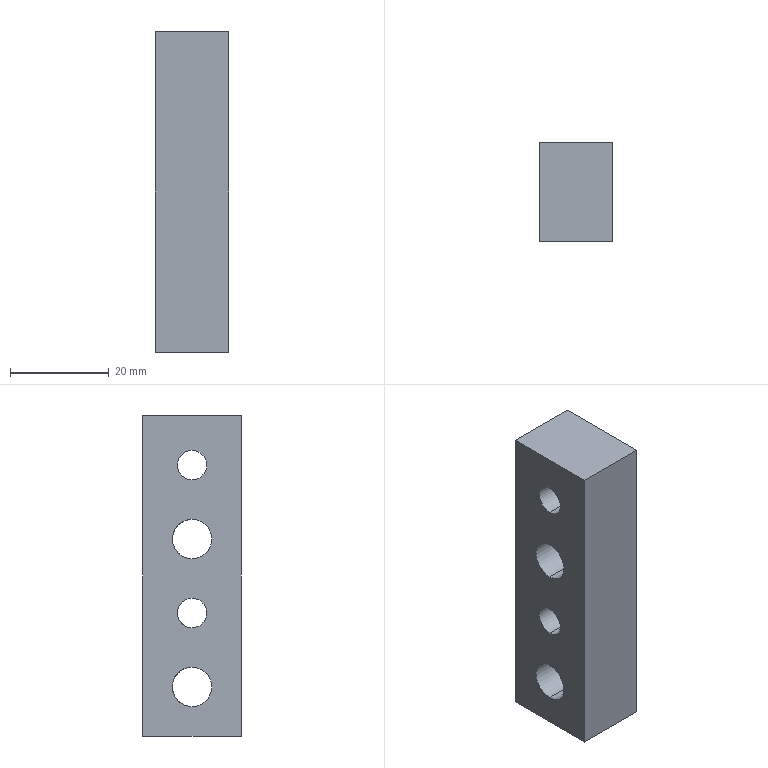Part | STEP file | Positioning_id1958_x_t | 1 solid | 14 faces | box 15 x 20 x 65 mm | volume 17144 mm3 | cylinder 8 | plane 6 | commonest cylinder face diameters 6 x4 8 x4
STEP:
#1=CARTESIAN_POINT('',(0.,0.,0.));
#2=DIRECTION('',(0.,0.,1.));
#3=DIRECTION('',(1.,0.,0.));
#4=AXIS2_PLACEMENT_3D('',#1,#2,#3);
#5=CARTESIAN_POINT('',(-702.002,-0.00002595,356.));
#6=VERTEX_POINT('',#5);
#7=CARTESIAN_POINT('',(-702.002,-0.00002595,348.));
#8=VERTEX_POINT('',#7);
#9=CARTESIAN_POINT('',(-702.002,-0.00002595,352.));
#10=DIRECTION('',(1.,0.,0.));
#11=DIRECTION('',(0.,0.,-1.));
#12=AXIS2_PLACEMENT_3D('',#9,#10,#11);
#13=CIRCLE('',#12,4.);
#14=CARTESIAN_POINT('',(-656.002,-0.00002595,352.));
#15=DIRECTION('',(1.,0.,0.));
#16=DIRECTION('',(0.,0.,1.));
#17=AXIS2_PLACEMENT_3D('',#14,#15,#16);
#18=CYLINDRICAL_SURFACE('',#17,4.);
#19=CARTESIAN_POINT('',(-3.142,-46.));
#20=DIRECTION('',(1.,0.));
#21=VECTOR('',#20,1.);
#22=LINE('',#19,#21);
#23=(GEOMETRIC_REPRESENTATION_CONTEXT(2)PARAMETRIC_REPRESENTATION_CONTEXT()REPRESENTATION_CONTEXT('',''));
#24=DEFINITIONAL_REPRESENTATION('',(#22),#23);
#25=PCURVE('',#18,#24);
#26=CARTESIAN_POINT('',(-702.002,-9.,411.));
#27=DIRECTION('',(-1.,0.,0.));
#28=DIRECTION('',(0.,-1.,0.));
#29=AXIS2_PLACEMENT_3D('',#26,#27,#28);
#30=PLANE('',#29);
#31=CARTESIAN_POINT('',(-9.,-63.));
#32=CARTESIAN_POINT('',(-15.928,-63.));
#33=CARTESIAN_POINT('',(-12.464,-57.));
#34=CARTESIAN_POINT('',(-9.,-51.));
#35=CARTESIAN_POINT('',(-5.536,-57.));
#36=CARTESIAN_POINT('',(-2.072,-63.));
#37=CARTESIAN_POINT('',(-9.,-63.));
#38=(BOUNDED_CURVE()B_SPLINE_CURVE(2,(#31,#32,#33,#34,#35,#36,#37),.UNSPECIFIED.,.T.,.F.)B_SPLINE_CURVE_WITH_KNOTS((1,2,2,2,2,1),(-2.094,0.,2.094,4.189,6.283,8.378),.UNSPECIFIED.)CURVE()GEOMETRIC_REPRESENTATION_ITEM()RATIONAL_B_SPLINE_CURVE((1.,0.5,1.,0.5,1.,0.5,1.))REPRESENTATION_ITEM(''));
#39=(GEOMETRIC_REPRESENTATION_CONTEXT(2)PARAMETRIC_REPRESENTATION_CONTEXT()REPRESENTATION_CONTEXT('',''));
#40=DEFINITIONAL_REPRESENTATION('',(#38),#39);
#41=PCURVE('',#30,#40);
#42=SURFACE_CURVE('',#13,(#25,#41),.PCURVE_S1.);
#43=EDGE_CURVE('',#6,#8,#42,.T.);
#44=ORIENTED_EDGE('',*,*,#43,.T.);
#45=CARTESIAN_POINT('',(-687.002,-0.00002595,348.));
#46=VERTEX_POINT('',#45);
#47=CARTESIAN_POINT('',(-687.002,-0.00002595,348.));
#48=DIRECTION('',(1.,0.,0.));
#49=VECTOR('',#48,1.);
#50=LINE('',#47,#49);
#51=CARTESIAN_POINT('',(3.142,-31.));
#52=DIRECTION('',(0.,1.));
#53=VECTOR('',#52,1.);
#54=LINE('',#51,#53);
#55=(GEOMETRIC_REPRESENTATION_CONTEXT(2)PARAMETRIC_REPRESENTATION_CONTEXT()REPRESENTATION_CONTEXT('',''));
#56=DEFINITIONAL_REPRESENTATION('',(#54),#55);
#57=PCURVE('',#18,#56);
#58=CARTESIAN_POINT('',(-656.002,-0.00002595,352.));
#59=DIRECTION('',(1.,0.,0.));
#60=DIRECTION('',(0.,0.,1.));
#61=AXIS2_PLACEMENT_3D('',#58,#59,#60);
#62=CYLINDRICAL_SURFACE('',#61,4.);
#63=CARTESIAN_POINT('',(3.142,-31.));
#64=DIRECTION('',(0.,1.));
#65=VECTOR('',#64,1.);
#66=LINE('',#63,#65);
#67=(GEOMETRIC_REPRESENTATION_CONTEXT(2)PARAMETRIC_REPRESENTATION_CONTEXT()REPRESENTATION_CONTEXT('',''));
#68=DEFINITIONAL_REPRESENTATION('',(#66),#67);
#69=PCURVE('',#62,#68);
#70=SURFACE_CURVE('',#50,(#57,#69),.PCURVE_S1.);
#71=EDGE_CURVE('',#8,#46,#70,.T.);
#72=ORIENTED_EDGE('',*,*,#71,.T.);
#73=CARTESIAN_POINT('',(-687.002,-0.00002595,356.));
#74=VERTEX_POINT('',#73);
#75=CARTESIAN_POINT('',(-687.002,-0.00002595,352.));
#76=DIRECTION('',(-1.,0.,0.));
#77=DIRECTION('',(0.,0.,-1.));
#78=AXIS2_PLACEMENT_3D('',#75,#76,#77);
#79=CIRCLE('',#78,4.);
#80=CARTESIAN_POINT('',(3.142,-31.));
#81=DIRECTION('',(-1.,0.));
#82=VECTOR('',#81,1.);
#83=LINE('',#80,#82);
#84=(GEOMETRIC_REPRESENTATION_CONTEXT(2)PARAMETRIC_REPRESENTATION_CONTEXT()REPRESENTATION_CONTEXT('',''));
#85=DEFINITIONAL_REPRESENTATION('',(#83),#84);
#86=PCURVE('',#18,#85);
#87=CARTESIAN_POINT('',(-687.002,-9.,411.));
#88=DIRECTION('',(1.,0.,0.));
#89=DIRECTION('',(0.,1.,0.));
#90=AXIS2_PLACEMENT_3D('',#87,#88,#89);
#91=PLANE('',#90);
#92=CARTESIAN_POINT('',(9.,-63.));
#93=CARTESIAN_POINT('',(2.072,-63.));
#94=CARTESIAN_POINT('',(5.536,-57.));
#95=CARTESIAN_POINT('',(9.,-51.));
#96=CARTESIAN_POINT('',(12.464,-57.));
#97=CARTESIAN_POINT('',(15.928,-63.));
#98=CARTESIAN_POINT('',(9.,-63.));
#99=(BOUNDED_CURVE()B_SPLINE_CURVE(2,(#92,#93,#94,#95,#96,#97,#98),.UNSPECIFIED.,.T.,.F.)B_SPLINE_CURVE_WITH_KNOTS((1,2,2,2,2,1),(-2.094,0.,2.094,4.189,6.283,8.378),.UNSPECIFIED.)CURVE()GEOMETRIC_REPRESENTATION_ITEM()RATIONAL_B_SPLINE_CURVE((1.,0.5,1.,0.5,1.,0.5,1.))REPRESENTATION_ITEM(''));
#100=(GEOMETRIC_REPRESENTATION_CONTEXT(2)PARAMETRIC_REPRESENTATION_CONTEXT()REPRESENTATION_CONTEXT('',''));
#101=DEFINITIONAL_REPRESENTATION('',(#99),#100);
#102=PCURVE('',#91,#101);
#103=SURFACE_CURVE('',#79,(#86,#102),.PCURVE_S1.);
#104=EDGE_CURVE('',#46,#74,#103,.T.);
#105=ORIENTED_EDGE('',*,*,#104,.T.);
#106=CARTESIAN_POINT('',(-687.002,-0.00002595,356.));
#107=DIRECTION('',(-1.,0.,0.));
#108=VECTOR('',#107,1.);
#109=LINE('',#106,#108);
#110=CARTESIAN_POINT('',(0.,-31.));
#111=DIRECTION('',(0.,-1.));
#112=VECTOR('',#111,1.);
#113=LINE('',#110,#112);
#114=(GEOMETRIC_REPRESENTATION_CONTEXT(2)PARAMETRIC_REPRESENTATION_CONTEXT()REPRESENTATION_CONTEXT('',''));
#115=DEFINITIONAL_REPRESENTATION('',(#113),#114);
#116=PCURVE('',#18,#115);
#117=CARTESIAN_POINT('',(6.283,-31.));
#118=DIRECTION('',(0.,-1.));
#119=VECTOR('',#118,1.);
#120=LINE('',#117,#119);
#121=(GEOMETRIC_REPRESENTATION_CONTEXT(2)PARAMETRIC_REPRESENTATION_CONTEXT()REPRESENTATION_CONTEXT('',''));
#122=DEFINITIONAL_REPRESENTATION('',(#120),#121);
#123=PCURVE('',#62,#122);
#124=SURFACE_CURVE('',#109,(#116,#123),.PCURVE_S1.);
#125=EDGE_CURVE('',#74,#6,#124,.T.);
#126=ORIENTED_EDGE('',*,*,#125,.T.);
#127=EDGE_LOOP('',(#44,#72,#105,#126));
#128=FACE_BOUND('',#127,.F.);
#129=ADVANCED_FACE('',(#128),#18,.F.);
#130=CARTESIAN_POINT('',(-702.002,-0.00002595,386.));
#131=VERTEX_POINT('',#130);
#132=CARTESIAN_POINT('',(-702.002,-0.00002595,378.));
#133=VERTEX_POINT('',#132);
#134=CARTESIAN_POINT('',(-702.002,-0.00002595,382.));
#135=DIRECTION('',(1.,0.,0.));
#136=DIRECTION('',(0.,0.,-1.));
#137=AXIS2_PLACEMENT_3D('',#134,#135,#136);
#138=CIRCLE('',#137,4.);
#139=CARTESIAN_POINT('',(-656.002,-0.00002595,382.));
#140=DIRECTION('',(1.,0.,0.));
#141=DIRECTION('',(0.,0.,1.));
#142=AXIS2_PLACEMENT_3D('',#139,#140,#141);
#143=CYLINDRICAL_SURFACE('',#142,4.);
#144=CARTESIAN_POINT('',(-3.142,-46.));
#145=DIRECTION('',(1.,0.));
#146=VECTOR('',#145,1.);
#147=LINE('',#144,#146);
#148=(GEOMETRIC_REPRESENTATION_CONTEXT(2)PARAMETRIC_REPRESENTATION_CONTEXT()REPRESENTATION_CONTEXT('',''));
#149=DEFINITIONAL_REPRESENTATION('',(#147),#148);
#150=PCURVE('',#143,#149);
#151=CARTESIAN_POINT('',(-9.,-33.));
#152=CARTESIAN_POINT('',(-15.928,-33.));
#153=CARTESIAN_POINT('',(-12.464,-27.));
#154=CARTESIAN_POINT('',(-9.,-21.));
#155=CARTESIAN_POINT('',(-5.536,-27.));
#156=CARTESIAN_POINT('',(-2.072,-33.));
#157=CARTESIAN_POINT('',(-9.,-33.));
#158=(BOUNDED_CURVE()B_SPLINE_CURVE(2,(#151,#152,#153,#154,#155,#156,#157),.UNSPECIFIED.,.T.,.F.)B_SPLINE_CURVE_WITH_KNOTS((1,2,2,2,2,1),(-2.094,0.,2.094,4.189,6.283,8.378),.UNSPECIFIED.)CURVE()GEOMETRIC_REPRESENTATION_ITEM()RATIONAL_B_SPLINE_CURVE((1.,0.5,1.,0.5,1.,0.5,1.))REPRESENTATION_ITEM(''));
#159=(GEOMETRIC_REPRESENTATION_CONTEXT(2)PARAMETRIC_REPRESENTATION_CONTEXT()REPRESENTATION_CONTEXT('',''));
#160=DEFINITIONAL_REPRESENTATION('',(#158),#159);
#161=PCURVE('',#30,#160);
#162=SURFACE_CURVE('',#138,(#150,#161),.PCURVE_S1.);
#163=EDGE_CURVE('',#131,#133,#162,.T.);
#164=ORIENTED_EDGE('',*,*,#163,.T.);
#165=CARTESIAN_POINT('',(-687.002,-0.00002595,378.));
#166=VERTEX_POINT('',#165);
#167=CARTESIAN_POINT('',(-687.002,-0.00002595,378.));
#168=DIRECTION('',(1.,0.,0.));
#169=VECTOR('',#168,1.);
#170=LINE('',#167,#169);
#171=CARTESIAN_POINT('',(3.142,-31.));
#172=DIRECTION('',(0.,1.));
#173=VECTOR('',#172,1.);
#174=LINE('',#171,#173);
#175=(GEOMETRIC_REPRESENTATION_CONTEXT(2)PARAMETRIC_REPRESENTATION_CONTEXT()REPRESENTATION_CONTEXT('',''));
#176=DEFINITIONAL_REPRESENTATION('',(#174),#175);
#177=PCURVE('',#143,#176);
#178=CARTESIAN_POINT('',(-656.002,-0.00002595,382.));
#179=DIRECTION('',(1.,0.,0.));
#180=DIRECTION('',(0.,0.,1.));
#181=AXIS2_PLACEMENT_3D('',#178,#179,#180);
#182=CYLINDRICAL_SURFACE('',#181,4.);
#183=CARTESIAN_POINT('',(3.142,-31.));
#184=DIRECTION('',(0.,1.));
#185=VECTOR('',#184,1.);
#186=LINE('',#183,#185);
#187=(GEOMETRIC_REPRESENTATION_CONTEXT(2)PARAMETRIC_REPRESENTATION_CONTEXT()REPRESENTATION_CONTEXT('',''));
#188=DEFINITIONAL_REPRESENTATION('',(#186),#187);
#189=PCURVE('',#182,#188);
#190=SURFACE_CURVE('',#170,(#177,#189),.PCURVE_S1.);
#191=EDGE_CURVE('',#133,#166,#190,.T.);
#192=ORIENTED_EDGE('',*,*,#191,.T.);
#193=CARTESIAN_POINT('',(-687.002,-0.00002595,386.));
#194=VERTEX_POINT('',#193);
#195=CARTESIAN_POINT('',(-687.002,-0.00002595,382.));
#196=DIRECTION('',(-1.,0.,0.));
#197=DIRECTION('',(0.,0.,-1.));
#198=AXIS2_PLACEMENT_3D('',#195,#196,#197);
#199=CIRCLE('',#198,4.);
#200=CARTESIAN_POINT('',(3.142,-31.));
#201=DIRECTION('',(-1.,0.));
#202=VECTOR('',#201,1.);
#203=LINE('',#200,#202);
#204=(GEOMETRIC_REPRESENTATION_CONTEXT(2)PARAMETRIC_REPRESENTATION_CONTEXT()REPRESENTATION_CONTEXT('',''));
#205=DEFINITIONAL_REPRESENTATION('',(#203),#204);
#206=PCURVE('',#143,#205);
#207=CARTESIAN_POINT('',(9.,-33.));
#208=CARTESIAN_POINT('',(2.072,-33.));
#209=CARTESIAN_POINT('',(5.536,-27.));
#210=CARTESIAN_POINT('',(9.,-21.));
#211=CARTESIAN_POINT('',(12.464,-27.));
#212=CARTESIAN_POINT('',(15.928,-33.));
#213=CARTESIAN_POINT('',(9.,-33.));
#214=(BOUNDED_CURVE()B_SPLINE_CURVE(2,(#207,#208,#209,#210,#211,#212,#213),.UNSPECIFIED.,.T.,.F.)B_SPLINE_CURVE_WITH_KNOTS((1,2,2,2,2,1),(-2.094,0.,2.094,4.189,6.283,8.378),.UNSPECIFIED.)CURVE()GEOMETRIC_REPRESENTATION_ITEM()RATIONAL_B_SPLINE_CURVE((1.,0.5,1.,0.5,1.,0.5,1.))REPRESENTATION_ITEM(''));
#215=(GEOMETRIC_REPRESENTATION_CONTEXT(2)PARAMETRIC_REPRESENTATION_CONTEXT()REPRESENTATION_CONTEXT('',''));
#216=DEFINITIONAL_REPRESENTATION('',(#214),#215);
#217=PCURVE('',#91,#216);
#218=SURFACE_CURVE('',#199,(#206,#217),.PCURVE_S1.);
#219=EDGE_CURVE('',#166,#194,#218,.T.);
#220=ORIENTED_EDGE('',*,*,#219,.T.);
#221=CARTESIAN_POINT('',(-687.002,-0.00002595,386.));
#222=DIRECTION('',(-1.,0.,0.));
#223=VECTOR('',#222,1.);
#224=LINE('',#221,#223);
#225=CARTESIAN_POINT('',(0.,-31.));
#226=DIRECTION('',(0.,-1.));
#227=VECTOR('',#226,1.);
#228=LINE('',#225,#227);
#229=(GEOMETRIC_REPRESENTATION_CONTEXT(2)PARAMETRIC_REPRESENTATION_CONTEXT()REPRESENTATION_CONTEXT('',''));
#230=DEFINITIONAL_REPRESENTATION('',(#228),#229);
#231=PCURVE('',#143,#230);
#232=CARTESIAN_POINT('',(6.283,-31.));
#233=DIRECTION('',(0.,-1.));
#234=VECTOR('',#233,1.);
#235=LINE('',#232,#234);
#236=(GEOMETRIC_REPRESENTATION_CONTEXT(2)PARAMETRIC_REPRESENTATION_CONTEXT()REPRESENTATION_CONTEXT('',''));
#237=DEFINITIONAL_REPRESENTATION('',(#235),#236);
#238=PCURVE('',#182,#237);
#239=SURFACE_CURVE('',#224,(#231,#238),.PCURVE_S1.);
#240=EDGE_CURVE('',#194,#131,#239,.T.);
#241=ORIENTED_EDGE('',*,*,#240,.T.);
#242=EDGE_LOOP('',(#164,#192,#220,#241));
#243=FACE_BOUND('',#242,.F.);
#244=ADVANCED_FACE('',(#243),#143,.F.);
#245=CARTESIAN_POINT('',(-702.002,-0.00002595,400.));
#246=VERTEX_POINT('',#245);
#247=CARTESIAN_POINT('',(-702.002,-0.00002595,394.));
#248=VERTEX_POINT('',#247);
#249=CARTESIAN_POINT('',(-702.002,-0.00002595,397.));
#250=DIRECTION('',(1.,0.,0.));
#251=DIRECTION('',(0.,0.,-1.));
#252=AXIS2_PLACEMENT_3D('',#249,#250,#251);
#253=CIRCLE('',#252,3.);
#254=CARTESIAN_POINT('',(-656.002,-0.00002595,397.));
#255=DIRECTION('',(1.,0.,0.));
#256=DIRECTION('',(0.,0.,1.));
#257=AXIS2_PLACEMENT_3D('',#254,#255,#256);
#258=CYLINDRICAL_SURFACE('',#257,3.);
#259=CARTESIAN_POINT('',(-3.142,-46.));
#260=DIRECTION('',(1.,0.));
#261=VECTOR('',#260,1.);
#262=LINE('',#259,#261);
#263=(GEOMETRIC_REPRESENTATION_CONTEXT(2)PARAMETRIC_REPRESENTATION_CONTEXT()REPRESENTATION_CONTEXT('',''));
#264=DEFINITIONAL_REPRESENTATION('',(#262),#263);
#265=PCURVE('',#258,#264);
#266=CARTESIAN_POINT('',(-9.,-17.));
#267=CARTESIAN_POINT('',(-14.196,-17.));
#268=CARTESIAN_POINT('',(-11.598,-12.5));
#269=CARTESIAN_POINT('',(-9.,-8.));
#270=CARTESIAN_POINT('',(-6.402,-12.5));
#271=CARTESIAN_POINT('',(-3.804,-17.));
#272=CARTESIAN_POINT('',(-9.,-17.));
#273=(BOUNDED_CURVE()B_SPLINE_CURVE(2,(#266,#267,#268,#269,#270,#271,#272),.UNSPECIFIED.,.T.,.F.)B_SPLINE_CURVE_WITH_KNOTS((1,2,2,2,2,1),(-2.094,0.,2.094,4.189,6.283,8.378),.UNSPECIFIED.)CURVE()GEOMETRIC_REPRESENTATION_ITEM()RATIONAL_B_SPLINE_CURVE((1.,0.5,1.,0.5,1.,0.5,1.))REPRESENTATION_ITEM(''));
#274=(GEOMETRIC_REPRESENTATION_CONTEXT(2)PARAMETRIC_REPRESENTATION_CONTEXT()REPRESENTATION_CONTEXT('',''));
#275=DEFINITIONAL_REPRESENTATION('',(#273),#274);
#276=PCURVE('',#30,#275);
#277=SURFACE_CURVE('',#253,(#265,#276),.PCURVE_S1.);
#278=EDGE_CURVE('',#246,#248,#277,.T.);
#279=ORIENTED_EDGE('',*,*,#278,.T.);
#280=CARTESIAN_POINT('',(-687.002,-0.00002595,394.));
#281=VERTEX_POINT('',#280);
#282=CARTESIAN_POINT('',(-687.002,-0.00002595,394.));
#283=DIRECTION('',(-1.,0.,0.));
#284=VECTOR('',#283,1.);
#285=LINE('',#282,#284);
#286=CARTESIAN_POINT('',(3.142,-31.));
#287=DIRECTION('',(0.,-1.));
#288=VECTOR('',#287,1.);
#289=LINE('',#286,#288);
#290=(GEOMETRIC_REPRESENTATION_CONTEXT(2)PARAMETRIC_REPRESENTATION_CONTEXT()REPRESENTATION_CONTEXT('',''));
#291=DEFINITIONAL_REPRESENTATION('',(#289),#290);
#292=PCURVE('',#258,#291);
#293=CARTESIAN_POINT('',(-656.002,-0.00002595,397.));
#294=DIRECTION('',(1.,0.,0.));
#295=DIRECTION('',(0.,0.,1.));
#296=AXIS2_PLACEMENT_3D('',#293,#294,#295);
#297=CYLINDRICAL_SURFACE('',#296,3.);
#298=CARTESIAN_POINT('',(3.142,-31.));
#299=DIRECTION('',(0.,-1.));
#300=VECTOR('',#299,1.);
#301=LINE('',#298,#300);
#302=(GEOMETRIC_REPRESENTATION_CONTEXT(2)PARAMETRIC_REPRESENTATION_CONTEXT()REPRESENTATION_CONTEXT('',''));
#303=DEFINITIONAL_REPRESENTATION('',(#301),#302);
#304=PCURVE('',#297,#303);
#305=SURFACE_CURVE('',#285,(#292,#304),.PCURVE_S1.);
#306=EDGE_CURVE('',#281,#248,#305,.T.);
#307=ORIENTED_EDGE('',*,*,#306,.F.);
#308=CARTESIAN_POINT('',(-687.002,-0.00002595,400.));
#309=VERTEX_POINT('',#308);
#310=CARTESIAN_POINT('',(-687.002,-0.00002595,397.));
#311=DIRECTION('',(-1.,0.,0.));
#312=DIRECTION('',(0.,0.,-1.));
#313=AXIS2_PLACEMENT_3D('',#310,#311,#312);
#314=CIRCLE('',#313,3.);
#315=CARTESIAN_POINT('',(3.142,-31.));
#316=DIRECTION('',(-1.,0.));
#317=VECTOR('',#316,1.);
#318=LINE('',#315,#317);
#319=(GEOMETRIC_REPRESENTATION_CONTEXT(2)PARAMETRIC_REPRESENTATION_CONTEXT()REPRESENTATION_CONTEXT('',''));
#320=DEFINITIONAL_REPRESENTATION('',(#318),#319);
#321=PCURVE('',#258,#320);
#322=CARTESIAN_POINT('',(9.,-17.));
#323=CARTESIAN_POINT('',(3.804,-17.));
#324=CARTESIAN_POINT('',(6.402,-12.5));
#325=CARTESIAN_POINT('',(9.,-8.));
#326=CARTESIAN_POINT('',(11.598,-12.5));
#327=CARTESIAN_POINT('',(14.196,-17.));
#328=CARTESIAN_POINT('',(9.,-17.));
#329=(BOUNDED_CURVE()B_SPLINE_CURVE(2,(#322,#323,#324,#325,#326,#327,#328),.UNSPECIFIED.,.T.,.F.)B_SPLINE_CURVE_WITH_KNOTS((1,2,2,2,2,1),(-2.094,0.,2.094,4.189,6.283,8.378),.UNSPECIFIED.)CURVE()GEOMETRIC_REPRESENTATION_ITEM()RATIONAL_B_SPLINE_CURVE((1.,0.5,1.,0.5,1.,0.5,1.))REPRESENTATION_ITEM(''));
#330=(GEOMETRIC_REPRESENTATION_CONTEXT(2)PARAMETRIC_REPRESENTATION_CONTEXT()REPRESENTATION_CONTEXT('',''));
#331=DEFINITIONAL_REPRESENTATION('',(#329),#330);
#332=PCURVE('',#91,#331);
#333=SURFACE_CURVE('',#314,(#321,#332),.PCURVE_S1.);
#334=EDGE_CURVE('',#281,#309,#333,.T.);
#335=ORIENTED_EDGE('',*,*,#334,.T.);
#336=CARTESIAN_POINT('',(-687.002,-0.00002595,400.));
#337=DIRECTION('',(1.,0.,0.));
#338=VECTOR('',#337,1.);
#339=LINE('',#336,#338);
#340=CARTESIAN_POINT('',(0.,-31.));
#341=DIRECTION('',(0.,1.));
#342=VECTOR('',#341,1.);
#343=LINE('',#340,#342);
#344=(GEOMETRIC_REPRESENTATION_CONTEXT(2)PARAMETRIC_REPRESENTATION_CONTEXT()REPRESENTATION_CONTEXT('',''));
#345=DEFINITIONAL_REPRESENTATION('',(#343),#344);
#346=PCURVE('',#258,#345);
#347=CARTESIAN_POINT('',(6.283,-31.));
#348=DIRECTION('',(0.,1.));
#349=VECTOR('',#348,1.);
#350=LINE('',#347,#349);
#351=(GEOMETRIC_REPRESENTATION_CONTEXT(2)PARAMETRIC_REPRESENTATION_CONTEXT()REPRESENTATION_CONTEXT('',''));
#352=DEFINITIONAL_REPRESENTATION('',(#350),#351);
#353=PCURVE('',#297,#352);
#354=SURFACE_CURVE('',#339,(#346,#353),.PCURVE_S1.);
#355=EDGE_CURVE('',#246,#309,#354,.T.);
#356=ORIENTED_EDGE('',*,*,#355,.F.);
#357=EDGE_LOOP('',(#279,#307,#335,#356));
#358=FACE_BOUND('',#357,.F.);
#359=ADVANCED_FACE('',(#358),#258,.F.);
#360=CARTESIAN_POINT('',(-702.002,-0.00002595,370.));
#361=VERTEX_POINT('',#360);
#362=CARTESIAN_POINT('',(-702.002,-0.00002595,364.));
#363=VERTEX_POINT('',#362);
#364=CARTESIAN_POINT('',(-702.002,-0.00002595,367.));
#365=DIRECTION('',(1.,0.,0.));
#366=DIRECTION('',(0.,0.,-1.));
#367=AXIS2_PLACEMENT_3D('',#364,#365,#366);
#368=CIRCLE('',#367,3.);
#369=CARTESIAN_POINT('',(-656.002,-0.00002595,367.));
#370=DIRECTION('',(1.,0.,0.));
#371=DIRECTION('',(0.,0.,1.));
#372=AXIS2_PLACEMENT_3D('',#369,#370,#371);
#373=CYLINDRICAL_SURFACE('',#372,3.);
#374=CARTESIAN_POINT('',(-3.142,-46.));
#375=DIRECTION('',(1.,0.));
#376=VECTOR('',#375,1.);
#377=LINE('',#374,#376);
#378=(GEOMETRIC_REPRESENTATION_CONTEXT(2)PARAMETRIC_REPRESENTATION_CONTEXT()REPRESENTATION_CONTEXT('',''));
#379=DEFINITIONAL_REPRESENTATION('',(#377),#378);
#380=PCURVE('',#373,#379);
#381=CARTESIAN_POINT('',(-9.,-47.));
#382=CARTESIAN_POINT('',(-14.196,-47.));
#383=CARTESIAN_POINT('',(-11.598,-42.5));
#384=CARTESIAN_POINT('',(-9.,-38.));
#385=CARTESIAN_POINT('',(-6.402,-42.5));
#386=CARTESIAN_POINT('',(-3.804,-47.));
#387=CARTESIAN_POINT('',(-9.,-47.));
#388=(BOUNDED_CURVE()B_SPLINE_CURVE(2,(#381,#382,#383,#384,#385,#386,#387),.UNSPECIFIED.,.T.,.F.)B_SPLINE_CURVE_WITH_KNOTS((1,2,2,2,2,1),(-2.094,0.,2.094,4.189,6.283,8.378),.UNSPECIFIED.)CURVE()GEOMETRIC_REPRESENTATION_ITEM()RATIONAL_B_SPLINE_CURVE((1.,0.5,1.,0.5,1.,0.5,1.))REPRESENTATION_ITEM(''));
#389=(GEOMETRIC_REPRESENTATION_CONTEXT(2)PARAMETRIC_REPRESENTATION_CONTEXT()REPRESENTATION_CONTEXT('',''));
#390=DEFINITIONAL_REPRESENTATION('',(#388),#389);
#391=PCURVE('',#30,#390);
#392=SURFACE_CURVE('',#368,(#380,#391),.PCURVE_S1.);
#393=EDGE_CURVE('',#361,#363,#392,.T.);
#394=ORIENTED_EDGE('',*,*,#393,.T.);
#395=CARTESIAN_POINT('',(-687.002,-0.00002595,364.));
#396=VERTEX_POINT('',#395);
#397=CARTESIAN_POINT('',(-687.002,-0.00002595,364.));
#398=DIRECTION('',(1.,0.,0.));
#399=VECTOR('',#398,1.);
#400=LINE('',#397,#399);
#401=CARTESIAN_POINT('',(3.142,-31.));
#402=DIRECTION('',(0.,1.));
#403=VECTOR('',#402,1.);
#404=LINE('',#401,#403);
#405=(GEOMETRIC_REPRESENTATION_CONTEXT(2)PARAMETRIC_REPRESENTATION_CONTEXT()REPRESENTATION_CONTEXT('',''));
#406=DEFINITIONAL_REPRESENTATION('',(#404),#405);
#407=PCURVE('',#373,#406);
#408=CARTESIAN_POINT('',(-656.002,-0.00002595,367.));
#409=DIRECTION('',(1.,0.,0.));
#410=DIRECTION('',(0.,0.,1.));
#411=AXIS2_PLACEMENT_3D('',#408,#409,#410);
#412=CYLINDRICAL_SURFACE('',#411,3.);
#413=CARTESIAN_POINT('',(3.142,-31.));
#414=DIRECTION('',(0.,1.));
#415=VECTOR('',#414,1.);
#416=LINE('',#413,#415);
#417=(GEOMETRIC_REPRESENTATION_CONTEXT(2)PARAMETRIC_REPRESENTATION_CONTEXT()REPRESENTATION_CONTEXT('',''));
#418=DEFINITIONAL_REPRESENTATION('',(#416),#417);
#419=PCURVE('',#412,#418);
#420=SURFACE_CURVE('',#400,(#407,#419),.PCURVE_S1.);
#421=EDGE_CURVE('',#363,#396,#420,.T.);
#422=ORIENTED_EDGE('',*,*,#421,.T.);
#423=CARTESIAN_POINT('',(-687.002,-0.00002595,370.));
#424=VERTEX_POINT('',#423);
#425=CARTESIAN_POINT('',(-687.002,-0.00002595,367.));
#426=DIRECTION('',(-1.,0.,0.));
#427=DIRECTION('',(0.,0.,-1.));
#428=AXIS2_PLACEMENT_3D('',#425,#426,#427);
#429=CIRCLE('',#428,3.);
#430=CARTESIAN_POINT('',(3.142,-31.));
#431=DIRECTION('',(-1.,0.));
#432=VECTOR('',#431,1.);
#433=LINE('',#430,#432);
#434=(GEOMETRIC_REPRESENTATION_CONTEXT(2)PARAMETRIC_REPRESENTATION_CONTEXT()REPRESENTATION_CONTEXT('',''));
#435=DEFINITIONAL_REPRESENTATION('',(#433),#434);
#436=PCURVE('',#373,#435);
#437=CARTESIAN_POINT('',(9.,-47.));
#438=CARTESIAN_POINT('',(3.804,-47.));
#439=CARTESIAN_POINT('',(6.402,-42.5));
#440=CARTESIAN_POINT('',(9.,-38.));
#441=CARTESIAN_POINT('',(11.598,-42.5));
#442=CARTESIAN_POINT('',(14.196,-47.));
#443=CARTESIAN_POINT('',(9.,-47.));
#444=(BOUNDED_CURVE()B_SPLINE_CURVE(2,(#437,#438,#439,#440,#441,#442,#443),.UNSPECIFIED.,.T.,.F.)B_SPLINE_CURVE_WITH_KNOTS((1,2,2,2,2,1),(-2.094,0.,2.094,4.189,6.283,8.378),.UNSPECIFIED.)CURVE()GEOMETRIC_REPRESENTATION_ITEM()RATIONAL_B_SPLINE_CURVE((1.,0.5,1.,0.5,1.,0.5,1.))REPRESENTATION_ITEM(''));
#445=(GEOMETRIC_REPRESENTATION_CONTEXT(2)PARAMETRIC_REPRESENTATION_CONTEXT()REPRESENTATION_CONTEXT('',''));
#446=DEFINITIONAL_REPRESENTATION('',(#444),#445);
#447=PCURVE('',#91,#446);
#448=SURFACE_CURVE('',#429,(#436,#447),.PCURVE_S1.);
#449=EDGE_CURVE('',#396,#424,#448,.T.);
#450=ORIENTED_EDGE('',*,*,#449,.T.);
#451=CARTESIAN_POINT('',(-687.002,-0.00002595,370.));
#452=DIRECTION('',(-1.,0.,0.));
#453=VECTOR('',#452,1.);
#454=LINE('',#451,#453);
#455=CARTESIAN_POINT('',(0.,-31.));
#456=DIRECTION('',(0.,-1.));
#457=VECTOR('',#456,1.);
#458=LINE('',#455,#457);
#459=(GEOMETRIC_REPRESENTATION_CONTEXT(2)PARAMETRIC_REPRESENTATION_CONTEXT()REPRESENTATION_CONTEXT('',''));
#460=DEFINITIONAL_REPRESENTATION('',(#458),#459);
#461=PCURVE('',#373,#460);
#462=CARTESIAN_POINT('',(6.283,-31.));
#463=DIRECTION('',(0.,-1.));
#464=VECTOR('',#463,1.);
#465=LINE('',#462,#464);
#466=(GEOMETRIC_REPRESENTATION_CONTEXT(2)PARAMETRIC_REPRESENTATION_CONTEXT()REPRESENTATION_CONTEXT('',''));
#467=DEFINITIONAL_REPRESENTATION('',(#465),#466);
#468=PCURVE('',#412,#467);
#469=SURFACE_CURVE('',#454,(#461,#468),.PCURVE_S1.);
#470=EDGE_CURVE('',#424,#361,#469,.T.);
#471=ORIENTED_EDGE('',*,*,#470,.T.);
#472=EDGE_LOOP('',(#394,#422,#450,#471));
#473=FACE_BOUND('',#472,.F.);
#474=ADVANCED_FACE('',(#473),#373,.F.);
#475=CARTESIAN_POINT('',(-702.002,10.,407.));
#476=VERTEX_POINT('',#475);
#477=CARTESIAN_POINT('',(-702.002,10.,342.));
#478=VERTEX_POINT('',#477);
#479=CARTESIAN_POINT('',(-702.002,10.,407.));
#480=DIRECTION('',(0.,0.,-1.));
#481=VECTOR('',#480,1.);
#482=LINE('',#479,#481);
#483=CARTESIAN_POINT('',(-697.002,10.,411.));
#484=DIRECTION('',(0.,1.,0.));
#485=DIRECTION('',(-1.,0.,0.));
#486=AXIS2_PLACEMENT_3D('',#483,#484,#485);
#487=PLANE('',#486);
#488=CARTESIAN_POINT('',(5.,-4.));
#489=DIRECTION('',(0.,-1.));
#490=VECTOR('',#489,1.);
#491=LINE('',#488,#490);
#492=(GEOMETRIC_REPRESENTATION_CONTEXT(2)PARAMETRIC_REPRESENTATION_CONTEXT()REPRESENTATION_CONTEXT('',''));
#493=DEFINITIONAL_REPRESENTATION('',(#491),#492);
#494=PCURVE('',#487,#493);
#495=CARTESIAN_POINT('',(-19.,-4.));
#496=DIRECTION('',(0.,-1.));
#497=VECTOR('',#496,1.);
#498=LINE('',#495,#497);
#499=(GEOMETRIC_REPRESENTATION_CONTEXT(2)PARAMETRIC_REPRESENTATION_CONTEXT()REPRESENTATION_CONTEXT('',''));
#500=DEFINITIONAL_REPRESENTATION('',(#498),#499);
#501=PCURVE('',#30,#500);
#502=SURFACE_CURVE('',#482,(#494,#501),.PCURVE_S1.);
#503=EDGE_CURVE('',#476,#478,#502,.T.);
#504=ORIENTED_EDGE('',*,*,#503,.F.);
#505=CARTESIAN_POINT('',(-687.002,10.,407.));
#506=VERTEX_POINT('',#505);
#507=CARTESIAN_POINT('',(-702.002,10.,407.));
#508=DIRECTION('',(1.,0.,0.));
#509=VECTOR('',#508,1.);
#510=LINE('',#507,#509);
#511=CARTESIAN_POINT('',(5.,-4.));
#512=DIRECTION('',(-1.,0.));
#513=VECTOR('',#512,1.);
#514=LINE('',#511,#513);
#515=(GEOMETRIC_REPRESENTATION_CONTEXT(2)PARAMETRIC_REPRESENTATION_CONTEXT()REPRESENTATION_CONTEXT('',''));
#516=DEFINITIONAL_REPRESENTATION('',(#514),#515);
#517=PCURVE('',#487,#516);
#518=CARTESIAN_POINT('',(-656.002,10.,407.));
#519=DIRECTION('',(0.,0.,1.));
#520=DIRECTION('',(0.,1.,0.));
#521=AXIS2_PLACEMENT_3D('',#518,#519,#520);
#522=PLANE('',#521);
#523=CARTESIAN_POINT('',(0.,46.));
#524=DIRECTION('',(0.,-1.));
#525=VECTOR('',#524,1.);
#526=LINE('',#523,#525);
#527=(GEOMETRIC_REPRESENTATION_CONTEXT(2)PARAMETRIC_REPRESENTATION_CONTEXT()REPRESENTATION_CONTEXT('',''));
#528=DEFINITIONAL_REPRESENTATION('',(#526),#527);
#529=PCURVE('',#522,#528);
#530=SURFACE_CURVE('',#510,(#517,#529),.PCURVE_S1.);
#531=EDGE_CURVE('',#476,#506,#530,.T.);
#532=ORIENTED_EDGE('',*,*,#531,.T.);
#533=CARTESIAN_POINT('',(-687.002,10.,342.));
#534=VERTEX_POINT('',#533);
#535=CARTESIAN_POINT('',(-687.002,10.,342.));
#536=DIRECTION('',(0.,0.,1.));
#537=VECTOR('',#536,1.);
#538=LINE('',#535,#537);
#539=CARTESIAN_POINT('',(-10.,-69.));
#540=DIRECTION('',(0.,1.));
#541=VECTOR('',#540,1.);
#542=LINE('',#539,#541);
#543=(GEOMETRIC_REPRESENTATION_CONTEXT(2)PARAMETRIC_REPRESENTATION_CONTEXT()REPRESENTATION_CONTEXT('',''));
#544=DEFINITIONAL_REPRESENTATION('',(#542),#543);
#545=PCURVE('',#487,#544);
#546=CARTESIAN_POINT('',(19.,-69.));
#547=DIRECTION('',(0.,1.));
#548=VECTOR('',#547,1.);
#549=LINE('',#546,#548);
#550=(GEOMETRIC_REPRESENTATION_CONTEXT(2)PARAMETRIC_REPRESENTATION_CONTEXT()REPRESENTATION_CONTEXT('',''));
#551=DEFINITIONAL_REPRESENTATION('',(#549),#550);
#552=PCURVE('',#91,#551);
#553=SURFACE_CURVE('',#538,(#545,#552),.PCURVE_S1.);
#554=EDGE_CURVE('',#534,#506,#553,.T.);
#555=ORIENTED_EDGE('',*,*,#554,.F.);
#556=CARTESIAN_POINT('',(-702.002,10.,342.));
#557=DIRECTION('',(1.,0.,0.));
#558=VECTOR('',#557,1.);
#559=LINE('',#556,#558);
#560=CARTESIAN_POINT('',(5.,-69.));
#561=DIRECTION('',(-1.,0.));
#562=VECTOR('',#561,1.);
#563=LINE('',#560,#562);
#564=(GEOMETRIC_REPRESENTATION_CONTEXT(2)PARAMETRIC_REPRESENTATION_CONTEXT()REPRESENTATION_CONTEXT('',''));
#565=DEFINITIONAL_REPRESENTATION('',(#563),#564);
#566=PCURVE('',#487,#565);
#567=CARTESIAN_POINT('',(-697.002,-9.,342.));
#568=DIRECTION('',(0.,0.,-1.));
#569=DIRECTION('',(0.,-1.,0.));
#570=AXIS2_PLACEMENT_3D('',#567,#568,#569);
#571=PLANE('',#570);
#572=CARTESIAN_POINT('',(-19.,5.));
#573=DIRECTION('',(0.,-1.));
#574=VECTOR('',#573,1.);
#575=LINE('',#572,#574);
#576=(GEOMETRIC_REPRESENTATION_CONTEXT(2)PARAMETRIC_REPRESENTATION_CONTEXT()REPRESENTATION_CONTEXT('',''));
#577=DEFINITIONAL_REPRESENTATION('',(#575),#576);
#578=PCURVE('',#571,#577);
#579=SURFACE_CURVE('',#559,(#566,#578),.PCURVE_S1.);
#580=EDGE_CURVE('',#478,#534,#579,.T.);
#581=ORIENTED_EDGE('',*,*,#580,.F.);
#582=EDGE_LOOP('',(#504,#532,#555,#581));
#583=FACE_BOUND('',#582,.T.);
#584=ADVANCED_FACE('',(#583),#487,.T.);
#585=CARTESIAN_POINT('',(-687.002,-10.,407.));
#586=VERTEX_POINT('',#585);
#587=CARTESIAN_POINT('',(-687.002,-10.,342.));
#588=VERTEX_POINT('',#587);
#589=CARTESIAN_POINT('',(-687.002,-10.,407.));
#590=DIRECTION('',(0.,0.,-1.));
#591=VECTOR('',#590,1.);
#592=LINE('',#589,#591);
#593=CARTESIAN_POINT('',(-697.002,-10.,411.));
#594=DIRECTION('',(0.,-1.,0.));
#595=DIRECTION('',(1.,0.,0.));
#596=AXIS2_PLACEMENT_3D('',#593,#594,#595);
#597=PLANE('',#596);
#598=CARTESIAN_POINT('',(10.,-4.));
#599=DIRECTION('',(0.,-1.));
#600=VECTOR('',#599,1.);
#601=LINE('',#598,#600);
#602=(GEOMETRIC_REPRESENTATION_CONTEXT(2)PARAMETRIC_REPRESENTATION_CONTEXT()REPRESENTATION_CONTEXT('',''));
#603=DEFINITIONAL_REPRESENTATION('',(#601),#602);
#604=PCURVE('',#597,#603);
#605=CARTESIAN_POINT('',(-1.,-4.));
#606=DIRECTION('',(0.,-1.));
#607=VECTOR('',#606,1.);
#608=LINE('',#605,#607);
#609=(GEOMETRIC_REPRESENTATION_CONTEXT(2)PARAMETRIC_REPRESENTATION_CONTEXT()REPRESENTATION_CONTEXT('',''));
#610=DEFINITIONAL_REPRESENTATION('',(#608),#609);
#611=PCURVE('',#91,#610);
#612=SURFACE_CURVE('',#592,(#604,#611),.PCURVE_S1.);
#613=EDGE_CURVE('',#586,#588,#612,.T.);
#614=ORIENTED_EDGE('',*,*,#613,.F.);
#615=CARTESIAN_POINT('',(-702.002,-10.,407.));
#616=VERTEX_POINT('',#615);
#617=CARTESIAN_POINT('',(-687.002,-10.,407.));
#618=DIRECTION('',(-1.,0.,0.));
#619=VECTOR('',#618,1.);
#620=LINE('',#617,#619);
#621=CARTESIAN_POINT('',(10.,-4.));
#622=DIRECTION('',(-1.,0.));
#623=VECTOR('',#622,1.);
#624=LINE('',#621,#623);
#625=(GEOMETRIC_REPRESENTATION_CONTEXT(2)PARAMETRIC_REPRESENTATION_CONTEXT()REPRESENTATION_CONTEXT('',''));
#626=DEFINITIONAL_REPRESENTATION('',(#624),#625);
#627=PCURVE('',#597,#626);
#628=CARTESIAN_POINT('',(-20.,31.));
#629=DIRECTION('',(0.,1.));
#630=VECTOR('',#629,1.);
#631=LINE('',#628,#630);
#632=(GEOMETRIC_REPRESENTATION_CONTEXT(2)PARAMETRIC_REPRESENTATION_CONTEXT()REPRESENTATION_CONTEXT('',''));
#633=DEFINITIONAL_REPRESENTATION('',(#631),#632);
#634=PCURVE('',#522,#633);
#635=SURFACE_CURVE('',#620,(#627,#634),.PCURVE_S1.);
#636=EDGE_CURVE('',#586,#616,#635,.T.);
#637=ORIENTED_EDGE('',*,*,#636,.T.);
#638=CARTESIAN_POINT('',(-702.002,-10.,342.));
#639=VERTEX_POINT('',#638);
#640=CARTESIAN_POINT('',(-702.002,-10.,342.));
#641=DIRECTION('',(0.,0.,1.));
#642=VECTOR('',#641,1.);
#643=LINE('',#640,#642);
#644=CARTESIAN_POINT('',(-5.,-69.));
#645=DIRECTION('',(0.,1.));
#646=VECTOR('',#645,1.);
#647=LINE('',#644,#646);
#648=(GEOMETRIC_REPRESENTATION_CONTEXT(2)PARAMETRIC_REPRESENTATION_CONTEXT()REPRESENTATION_CONTEXT('',''));
#649=DEFINITIONAL_REPRESENTATION('',(#647),#648);
#650=PCURVE('',#597,#649);
#651=CARTESIAN_POINT('',(1.,-69.));
#652=DIRECTION('',(0.,1.));
#653=VECTOR('',#652,1.);
#654=LINE('',#651,#653);
#655=(GEOMETRIC_REPRESENTATION_CONTEXT(2)PARAMETRIC_REPRESENTATION_CONTEXT()REPRESENTATION_CONTEXT('',''));
#656=DEFINITIONAL_REPRESENTATION('',(#654),#655);
#657=PCURVE('',#30,#656);
#658=SURFACE_CURVE('',#643,(#650,#657),.PCURVE_S1.);
#659=EDGE_CURVE('',#639,#616,#658,.T.);
#660=ORIENTED_EDGE('',*,*,#659,.F.);
#661=CARTESIAN_POINT('',(-687.002,-10.,342.));
#662=DIRECTION('',(-1.,0.,0.));
#663=VECTOR('',#662,1.);
#664=LINE('',#661,#663);
#665=CARTESIAN_POINT('',(10.,-69.));
#666=DIRECTION('',(-1.,0.));
#667=VECTOR('',#666,1.);
#668=LINE('',#665,#667);
#669=(GEOMETRIC_REPRESENTATION_CONTEXT(2)PARAMETRIC_REPRESENTATION_CONTEXT()REPRESENTATION_CONTEXT('',''));
#670=DEFINITIONAL_REPRESENTATION('',(#668),#669);
#671=PCURVE('',#597,#670);
#672=CARTESIAN_POINT('',(1.,-10.));
#673=DIRECTION('',(0.,1.));
#674=VECTOR('',#673,1.);
#675=LINE('',#672,#674);
#676=(GEOMETRIC_REPRESENTATION_CONTEXT(2)PARAMETRIC_REPRESENTATION_CONTEXT()REPRESENTATION_CONTEXT('',''));
#677=DEFINITIONAL_REPRESENTATION('',(#675),#676);
#678=PCURVE('',#571,#677);
#679=SURFACE_CURVE('',#664,(#671,#678),.PCURVE_S1.);
#680=EDGE_CURVE('',#588,#639,#679,.T.);
#681=ORIENTED_EDGE('',*,*,#680,.F.);
#682=EDGE_LOOP('',(#614,#637,#660,#681));
#683=FACE_BOUND('',#682,.T.);
#684=ADVANCED_FACE('',(#683),#597,.T.);
#685=ORIENTED_EDGE('',*,*,#449,.T.);
#686=CARTESIAN_POINT('',(-687.002,-0.00002595,370.));
#687=CARTESIAN_POINT('',(-687.002,3.,370.));
#688=CARTESIAN_POINT('',(-687.002,4.5,367.));
#689=CARTESIAN_POINT('',(-687.002,3.,364.));
#690=CARTESIAN_POINT('',(-687.002,-0.00002595,364.));
#691=(BOUNDED_CURVE()B_SPLINE_CURVE(4,(#686,#687,#688,#689,#690),.UNSPECIFIED.,.F.,.F.)B_SPLINE_CURVE_WITH_KNOTS((5,5),(0.,1.),.PIECEWISE_BEZIER_KNOTS.)CURVE()GEOMETRIC_REPRESENTATION_ITEM()RATIONAL_B_SPLINE_CURVE((1.,0.7071,0.6667,0.7071,1.))REPRESENTATION_ITEM(''));
#692=CARTESIAN_POINT('',(9.,-41.));
#693=CARTESIAN_POINT('',(12.,-41.));
#694=CARTESIAN_POINT('',(13.5,-44.));
#695=CARTESIAN_POINT('',(12.,-47.));
#696=CARTESIAN_POINT('',(9.,-47.));
#697=(BOUNDED_CURVE()B_SPLINE_CURVE(4,(#692,#693,#694,#695,#696),.UNSPECIFIED.,.F.,.F.)B_SPLINE_CURVE_WITH_KNOTS((5,5),(0.,1.),.PIECEWISE_BEZIER_KNOTS.)CURVE()GEOMETRIC_REPRESENTATION_ITEM()RATIONAL_B_SPLINE_CURVE((1.,0.7071,0.6667,0.7071,1.))REPRESENTATION_ITEM(''));
#698=(GEOMETRIC_REPRESENTATION_CONTEXT(2)PARAMETRIC_REPRESENTATION_CONTEXT()REPRESENTATION_CONTEXT('',''));
#699=DEFINITIONAL_REPRESENTATION('',(#697),#698);
#700=PCURVE('',#91,#699);
#701=CARTESIAN_POINT('',(6.283,-31.));
#702=CARTESIAN_POINT('',(6.24,-31.));
#703=CARTESIAN_POINT('',(6.153,-31.));
#704=CARTESIAN_POINT('',(6.02,-31.));
#705=CARTESIAN_POINT('',(5.883,-31.));
#706=CARTESIAN_POINT('',(5.744,-31.));
#707=CARTESIAN_POINT('',(5.602,-31.));
#708=CARTESIAN_POINT('',(5.457,-31.));
#709=CARTESIAN_POINT('',(5.311,-31.));
#710=CARTESIAN_POINT('',(5.163,-31.));
#711=CARTESIAN_POINT('',(5.013,-31.));
#712=CARTESIAN_POINT('',(4.863,-31.));
#713=CARTESIAN_POINT('',(4.712,-31.));
#714=CARTESIAN_POINT('',(4.562,-31.));
#715=CARTESIAN_POINT('',(4.412,-31.));
#716=CARTESIAN_POINT('',(4.262,-31.));
#717=CARTESIAN_POINT('',(4.114,-31.));
#718=CARTESIAN_POINT('',(3.968,-31.));
#719=CARTESIAN_POINT('',(3.823,-31.));
#720=CARTESIAN_POINT('',(3.681,-31.));
#721=CARTESIAN_POINT('',(3.542,-31.));
#722=CARTESIAN_POINT('',(3.405,-31.));
#723=CARTESIAN_POINT('',(3.271,-31.));
#724=CARTESIAN_POINT('',(3.184,-31.));
#725=CARTESIAN_POINT('',(3.142,-31.));
#726=B_SPLINE_CURVE_WITH_KNOTS('',3,(#701,#702,#703,#704,#705,#706,#707,#708,#709,#710,#711,#712,#713,#714,#715,#716,#717,#718,#719,#720,#721,#722,#723,#724,#725),.UNSPECIFIED.,.F.,.F.,(4,1,1,1,1,1,1,1,1,1,1,1,1,1,1,1,1,1,1,1,1,1,4),(0.,0.04545,0.09091,0.1364,0.1818,0.2273,0.2727,0.3182,0.3636,0.4091,0.4545,0.5,0.5455,0.5909,0.6364,0.6818,0.7273,0.7727,0.8182,0.8636,0.9091,0.9545,1.),.QUASI_UNIFORM_KNOTS.);
#727=(GEOMETRIC_REPRESENTATION_CONTEXT(2)PARAMETRIC_REPRESENTATION_CONTEXT()REPRESENTATION_CONTEXT('',''));
#728=DEFINITIONAL_REPRESENTATION('',(#726),#727);
#729=PCURVE('',#412,#728);
#730=SURFACE_CURVE('',#691,(#700,#729),.PCURVE_S1.);
#731=EDGE_CURVE('',#424,#396,#730,.T.);
#732=ORIENTED_EDGE('',*,*,#731,.T.);
#733=EDGE_LOOP('',(#685,#732));
#734=FACE_BOUND('',#733,.T.);
#735=ORIENTED_EDGE('',*,*,#334,.T.);
#736=CARTESIAN_POINT('',(-687.002,-0.00002595,400.));
#737=CARTESIAN_POINT('',(-687.002,3.,400.));
#738=CARTESIAN_POINT('',(-687.002,4.5,397.));
#739=CARTESIAN_POINT('',(-687.002,3.,394.));
#740=CARTESIAN_POINT('',(-687.002,-0.00002595,394.));
#741=(BOUNDED_CURVE()B_SPLINE_CURVE(4,(#736,#737,#738,#739,#740),.UNSPECIFIED.,.F.,.F.)B_SPLINE_CURVE_WITH_KNOTS((5,5),(0.,1.),.PIECEWISE_BEZIER_KNOTS.)CURVE()GEOMETRIC_REPRESENTATION_ITEM()RATIONAL_B_SPLINE_CURVE((1.,0.7071,0.6667,0.7071,1.))REPRESENTATION_ITEM(''));
#742=CARTESIAN_POINT('',(9.,-11.));
#743=CARTESIAN_POINT('',(12.,-11.));
#744=CARTESIAN_POINT('',(13.5,-14.));
#745=CARTESIAN_POINT('',(12.,-17.));
#746=CARTESIAN_POINT('',(9.,-17.));
#747=(BOUNDED_CURVE()B_SPLINE_CURVE(4,(#742,#743,#744,#745,#746),.UNSPECIFIED.,.F.,.F.)B_SPLINE_CURVE_WITH_KNOTS((5,5),(0.,1.),.PIECEWISE_BEZIER_KNOTS.)CURVE()GEOMETRIC_REPRESENTATION_ITEM()RATIONAL_B_SPLINE_CURVE((1.,0.7071,0.6667,0.7071,1.))REPRESENTATION_ITEM(''));
#748=(GEOMETRIC_REPRESENTATION_CONTEXT(2)PARAMETRIC_REPRESENTATION_CONTEXT()REPRESENTATION_CONTEXT('',''));
#749=DEFINITIONAL_REPRESENTATION('',(#747),#748);
#750=PCURVE('',#91,#749);
#751=CARTESIAN_POINT('',(6.283,-31.));
#752=CARTESIAN_POINT('',(6.24,-31.));
#753=CARTESIAN_POINT('',(6.153,-31.));
#754=CARTESIAN_POINT('',(6.02,-31.));
#755=CARTESIAN_POINT('',(5.883,-31.));
#756=CARTESIAN_POINT('',(5.744,-31.));
#757=CARTESIAN_POINT('',(5.602,-31.));
#758=CARTESIAN_POINT('',(5.457,-31.));
#759=CARTESIAN_POINT('',(5.311,-31.));
#760=CARTESIAN_POINT('',(5.163,-31.));
#761=CARTESIAN_POINT('',(5.013,-31.));
#762=CARTESIAN_POINT('',(4.863,-31.));
#763=CARTESIAN_POINT('',(4.712,-31.));
#764=CARTESIAN_POINT('',(4.562,-31.));
#765=CARTESIAN_POINT('',(4.412,-31.));
#766=CARTESIAN_POINT('',(4.262,-31.));
#767=CARTESIAN_POINT('',(4.114,-31.));
#768=CARTESIAN_POINT('',(3.968,-31.));
#769=CARTESIAN_POINT('',(3.823,-31.));
#770=CARTESIAN_POINT('',(3.681,-31.));
#771=CARTESIAN_POINT('',(3.542,-31.));
#772=CARTESIAN_POINT('',(3.405,-31.));
#773=CARTESIAN_POINT('',(3.271,-31.));
#774=CARTESIAN_POINT('',(3.184,-31.));
#775=CARTESIAN_POINT('',(3.142,-31.));
#776=B_SPLINE_CURVE_WITH_KNOTS('',3,(#751,#752,#753,#754,#755,#756,#757,#758,#759,#760,#761,#762,#763,#764,#765,#766,#767,#768,#769,#770,#771,#772,#773,#774,#775),.UNSPECIFIED.,.F.,.F.,(4,1,1,1,1,1,1,1,1,1,1,1,1,1,1,1,1,1,1,1,1,1,4),(0.,0.04545,0.09091,0.1364,0.1818,0.2273,0.2727,0.3182,0.3636,0.4091,0.4545,0.5,0.5455,0.5909,0.6364,0.6818,0.7273,0.7727,0.8182,0.8636,0.9091,0.9545,1.),.QUASI_UNIFORM_KNOTS.);
#777=(GEOMETRIC_REPRESENTATION_CONTEXT(2)PARAMETRIC_REPRESENTATION_CONTEXT()REPRESENTATION_CONTEXT('',''));
#778=DEFINITIONAL_REPRESENTATION('',(#776),#777);
#779=PCURVE('',#297,#778);
#780=SURFACE_CURVE('',#741,(#750,#779),.PCURVE_S1.);
#781=EDGE_CURVE('',#309,#281,#780,.T.);
#782=ORIENTED_EDGE('',*,*,#781,.T.);
#783=EDGE_LOOP('',(#735,#782));
#784=FACE_BOUND('',#783,.T.);
#785=ORIENTED_EDGE('',*,*,#219,.T.);
#786=CARTESIAN_POINT('',(-687.002,-0.00002595,386.));
#787=CARTESIAN_POINT('',(-687.002,4.,386.));
#788=CARTESIAN_POINT('',(-687.002,6.,382.));
#789=CARTESIAN_POINT('',(-687.002,4.,378.));
#790=CARTESIAN_POINT('',(-687.002,-0.00002595,378.));
#791=(BOUNDED_CURVE()B_SPLINE_CURVE(4,(#786,#787,#788,#789,#790),.UNSPECIFIED.,.F.,.F.)B_SPLINE_CURVE_WITH_KNOTS((5,5),(0.,1.),.PIECEWISE_BEZIER_KNOTS.)CURVE()GEOMETRIC_REPRESENTATION_ITEM()RATIONAL_B_SPLINE_CURVE((1.,0.7071,0.6667,0.7071,1.))REPRESENTATION_ITEM(''));
#792=CARTESIAN_POINT('',(9.,-25.));
#793=CARTESIAN_POINT('',(13.,-25.));
#794=CARTESIAN_POINT('',(15.,-29.));
#795=CARTESIAN_POINT('',(13.,-33.));
#796=CARTESIAN_POINT('',(9.,-33.));
#797=(BOUNDED_CURVE()B_SPLINE_CURVE(4,(#792,#793,#794,#795,#796),.UNSPECIFIED.,.F.,.F.)B_SPLINE_CURVE_WITH_KNOTS((5,5),(0.,1.),.PIECEWISE_BEZIER_KNOTS.)CURVE()GEOMETRIC_REPRESENTATION_ITEM()RATIONAL_B_SPLINE_CURVE((1.,0.7071,0.6667,0.7071,1.))REPRESENTATION_ITEM(''));
#798=(GEOMETRIC_REPRESENTATION_CONTEXT(2)PARAMETRIC_REPRESENTATION_CONTEXT()REPRESENTATION_CONTEXT('',''));
#799=DEFINITIONAL_REPRESENTATION('',(#797),#798);
#800=PCURVE('',#91,#799);
#801=CARTESIAN_POINT('',(6.283,-31.));
#802=CARTESIAN_POINT('',(6.24,-31.));
#803=CARTESIAN_POINT('',(6.153,-31.));
#804=CARTESIAN_POINT('',(6.02,-31.));
#805=CARTESIAN_POINT('',(5.883,-31.));
#806=CARTESIAN_POINT('',(5.744,-31.));
#807=CARTESIAN_POINT('',(5.602,-31.));
#808=CARTESIAN_POINT('',(5.457,-31.));
#809=CARTESIAN_POINT('',(5.311,-31.));
#810=CARTESIAN_POINT('',(5.163,-31.));
#811=CARTESIAN_POINT('',(5.013,-31.));
#812=CARTESIAN_POINT('',(4.863,-31.));
#813=CARTESIAN_POINT('',(4.712,-31.));
#814=CARTESIAN_POINT('',(4.562,-31.));
#815=CARTESIAN_POINT('',(4.412,-31.));
#816=CARTESIAN_POINT('',(4.262,-31.));
#817=CARTESIAN_POINT('',(4.114,-31.));
#818=CARTESIAN_POINT('',(3.968,-31.));
#819=CARTESIAN_POINT('',(3.823,-31.));
#820=CARTESIAN_POINT('',(3.681,-31.));
#821=CARTESIAN_POINT('',(3.542,-31.));
#822=CARTESIAN_POINT('',(3.405,-31.));
#823=CARTESIAN_POINT('',(3.271,-31.));
#824=CARTESIAN_POINT('',(3.184,-31.));
#825=CARTESIAN_POINT('',(3.142,-31.));
#826=B_SPLINE_CURVE_WITH_KNOTS('',3,(#801,#802,#803,#804,#805,#806,#807,#808,#809,#810,#811,#812,#813,#814,#815,#816,#817,#818,#819,#820,#821,#822,#823,#824,#825),.UNSPECIFIED.,.F.,.F.,(4,1,1,1,1,1,1,1,1,1,1,1,1,1,1,1,1,1,1,1,1,1,4),(0.,0.04545,0.09091,0.1364,0.1818,0.2273,0.2727,0.3182,0.3636,0.4091,0.4545,0.5,0.5455,0.5909,0.6364,0.6818,0.7273,0.7727,0.8182,0.8636,0.9091,0.9545,1.),.QUASI_UNIFORM_KNOTS.);
#827=(GEOMETRIC_REPRESENTATION_CONTEXT(2)PARAMETRIC_REPRESENTATION_CONTEXT()REPRESENTATION_CONTEXT('',''));
#828=DEFINITIONAL_REPRESENTATION('',(#826),#827);
#829=PCURVE('',#182,#828);
#830=SURFACE_CURVE('',#791,(#800,#829),.PCURVE_S1.);
#831=EDGE_CURVE('',#194,#166,#830,.T.);
#832=ORIENTED_EDGE('',*,*,#831,.T.);
#833=EDGE_LOOP('',(#785,#832));
#834=FACE_BOUND('',#833,.T.);
#835=ORIENTED_EDGE('',*,*,#104,.T.);
#836=CARTESIAN_POINT('',(-687.002,-0.00002595,356.));
#837=CARTESIAN_POINT('',(-687.002,4.,356.));
#838=CARTESIAN_POINT('',(-687.002,6.,352.));
#839=CARTESIAN_POINT('',(-687.002,4.,348.));
#840=CARTESIAN_POINT('',(-687.002,-0.00002595,348.));
#841=(BOUNDED_CURVE()B_SPLINE_CURVE(4,(#836,#837,#838,#839,#840),.UNSPECIFIED.,.F.,.F.)B_SPLINE_CURVE_WITH_KNOTS((5,5),(0.,1.),.PIECEWISE_BEZIER_KNOTS.)CURVE()GEOMETRIC_REPRESENTATION_ITEM()RATIONAL_B_SPLINE_CURVE((1.,0.7071,0.6667,0.7071,1.))REPRESENTATION_ITEM(''));
#842=CARTESIAN_POINT('',(9.,-55.));
#843=CARTESIAN_POINT('',(13.,-55.));
#844=CARTESIAN_POINT('',(15.,-59.));
#845=CARTESIAN_POINT('',(13.,-63.));
#846=CARTESIAN_POINT('',(9.,-63.));
#847=(BOUNDED_CURVE()B_SPLINE_CURVE(4,(#842,#843,#844,#845,#846),.UNSPECIFIED.,.F.,.F.)B_SPLINE_CURVE_WITH_KNOTS((5,5),(0.,1.),.PIECEWISE_BEZIER_KNOTS.)CURVE()GEOMETRIC_REPRESENTATION_ITEM()RATIONAL_B_SPLINE_CURVE((1.,0.7071,0.6667,0.7071,1.))REPRESENTATION_ITEM(''));
#848=(GEOMETRIC_REPRESENTATION_CONTEXT(2)PARAMETRIC_REPRESENTATION_CONTEXT()REPRESENTATION_CONTEXT('',''));
#849=DEFINITIONAL_REPRESENTATION('',(#847),#848);
#850=PCURVE('',#91,#849);
#851=CARTESIAN_POINT('',(6.283,-31.));
#852=CARTESIAN_POINT('',(6.24,-31.));
#853=CARTESIAN_POINT('',(6.153,-31.));
#854=CARTESIAN_POINT('',(6.02,-31.));
#855=CARTESIAN_POINT('',(5.883,-31.));
#856=CARTESIAN_POINT('',(5.744,-31.));
#857=CARTESIAN_POINT('',(5.602,-31.));
#858=CARTESIAN_POINT('',(5.457,-31.));
#859=CARTESIAN_POINT('',(5.311,-31.));
#860=CARTESIAN_POINT('',(5.163,-31.));
#861=CARTESIAN_POINT('',(5.013,-31.));
#862=CARTESIAN_POINT('',(4.863,-31.));
#863=CARTESIAN_POINT('',(4.712,-31.));
#864=CARTESIAN_POINT('',(4.562,-31.));
#865=CARTESIAN_POINT('',(4.412,-31.));
#866=CARTESIAN_POINT('',(4.262,-31.));
#867=CARTESIAN_POINT('',(4.114,-31.));
#868=CARTESIAN_POINT('',(3.968,-31.));
#869=CARTESIAN_POINT('',(3.823,-31.));
#870=CARTESIAN_POINT('',(3.681,-31.));
#871=CARTESIAN_POINT('',(3.542,-31.));
#872=CARTESIAN_POINT('',(3.405,-31.));
#873=CARTESIAN_POINT('',(3.271,-31.));
#874=CARTESIAN_POINT('',(3.184,-31.));
#875=CARTESIAN_POINT('',(3.142,-31.));
#876=B_SPLINE_CURVE_WITH_KNOTS('',3,(#851,#852,#853,#854,#855,#856,#857,#858,#859,#860,#861,#862,#863,#864,#865,#866,#867,#868,#869,#870,#871,#872,#873,#874,#875),.UNSPECIFIED.,.F.,.F.,(4,1,1,1,1,1,1,1,1,1,1,1,1,1,1,1,1,1,1,1,1,1,4),(0.,0.04545,0.09091,0.1364,0.1818,0.2273,0.2727,0.3182,0.3636,0.4091,0.4545,0.5,0.5455,0.5909,0.6364,0.6818,0.7273,0.7727,0.8182,0.8636,0.9091,0.9545,1.),.QUASI_UNIFORM_KNOTS.);
#877=(GEOMETRIC_REPRESENTATION_CONTEXT(2)PARAMETRIC_REPRESENTATION_CONTEXT()REPRESENTATION_CONTEXT('',''));
#878=DEFINITIONAL_REPRESENTATION('',(#876),#877);
#879=PCURVE('',#62,#878);
#880=SURFACE_CURVE('',#841,(#850,#879),.PCURVE_S1.);
#881=EDGE_CURVE('',#74,#46,#880,.T.);
#882=ORIENTED_EDGE('',*,*,#881,.T.);
#883=EDGE_LOOP('',(#835,#882));
#884=FACE_BOUND('',#883,.T.);
#885=ORIENTED_EDGE('',*,*,#554,.T.);
#886=CARTESIAN_POINT('',(-687.002,10.,407.));
#887=DIRECTION('',(0.,-1.,0.));
#888=VECTOR('',#887,1.);
#889=LINE('',#886,#888);
#890=CARTESIAN_POINT('',(19.,-4.));
#891=DIRECTION('',(-1.,0.));
#892=VECTOR('',#891,1.);
#893=LINE('',#890,#892);
#894=(GEOMETRIC_REPRESENTATION_CONTEXT(2)PARAMETRIC_REPRESENTATION_CONTEXT()REPRESENTATION_CONTEXT('',''));
#895=DEFINITIONAL_REPRESENTATION('',(#893),#894);
#896=PCURVE('',#91,#895);
#897=CARTESIAN_POINT('',(0.,31.));
#898=DIRECTION('',(-1.,0.));
#899=VECTOR('',#898,1.);
#900=LINE('',#897,#899);
#901=(GEOMETRIC_REPRESENTATION_CONTEXT(2)PARAMETRIC_REPRESENTATION_CONTEXT()REPRESENTATION_CONTEXT('',''));
#902=DEFINITIONAL_REPRESENTATION('',(#900),#901);
#903=PCURVE('',#522,#902);
#904=SURFACE_CURVE('',#889,(#896,#903),.PCURVE_S1.);
#905=EDGE_CURVE('',#506,#586,#904,.T.);
#906=ORIENTED_EDGE('',*,*,#905,.T.);
#907=ORIENTED_EDGE('',*,*,#613,.T.);
#908=CARTESIAN_POINT('',(-687.002,-10.,342.));
#909=DIRECTION('',(0.,1.,0.));
#910=VECTOR('',#909,1.);
#911=LINE('',#908,#910);
#912=CARTESIAN_POINT('',(-1.,-69.));
#913=DIRECTION('',(1.,0.));
#914=VECTOR('',#913,1.);
#915=LINE('',#912,#914);
#916=(GEOMETRIC_REPRESENTATION_CONTEXT(2)PARAMETRIC_REPRESENTATION_CONTEXT()REPRESENTATION_CONTEXT('',''));
#917=DEFINITIONAL_REPRESENTATION('',(#915),#916);
#918=PCURVE('',#91,#917);
#919=CARTESIAN_POINT('',(1.,-10.));
#920=DIRECTION('',(-1.,0.));
#921=VECTOR('',#920,1.);
#922=LINE('',#919,#921);
#923=(GEOMETRIC_REPRESENTATION_CONTEXT(2)PARAMETRIC_REPRESENTATION_CONTEXT()REPRESENTATION_CONTEXT('',''));
#924=DEFINITIONAL_REPRESENTATION('',(#922),#923);
#925=PCURVE('',#571,#924);
#926=SURFACE_CURVE('',#911,(#918,#925),.PCURVE_S1.);
#927=EDGE_CURVE('',#588,#534,#926,.T.);
#928=ORIENTED_EDGE('',*,*,#927,.T.);
#929=EDGE_LOOP('',(#885,#906,#907,#928));
#930=FACE_BOUND('',#929,.T.);
#931=ADVANCED_FACE('',(#734,#784,#834,#884,#930),#91,.T.);
#932=CARTESIAN_POINT('',(-702.002,-10.,342.));
#933=DIRECTION('',(0.,1.,0.));
#934=VECTOR('',#933,1.);
#935=LINE('',#932,#934);
#936=CARTESIAN_POINT('',(1.,5.));
#937=DIRECTION('',(-1.,0.));
#938=VECTOR('',#937,1.);
#939=LINE('',#936,#938);
#940=(GEOMETRIC_REPRESENTATION_CONTEXT(2)PARAMETRIC_REPRESENTATION_CONTEXT()REPRESENTATION_CONTEXT('',''));
#941=DEFINITIONAL_REPRESENTATION('',(#939),#940);
#942=PCURVE('',#571,#941);
#943=CARTESIAN_POINT('',(1.,-69.));
#944=DIRECTION('',(-1.,0.));
#945=VECTOR('',#944,1.);
#946=LINE('',#943,#945);
#947=(GEOMETRIC_REPRESENTATION_CONTEXT(2)PARAMETRIC_REPRESENTATION_CONTEXT()REPRESENTATION_CONTEXT('',''));
#948=DEFINITIONAL_REPRESENTATION('',(#946),#947);
#949=PCURVE('',#30,#948);
#950=SURFACE_CURVE('',#935,(#942,#949),.PCURVE_S1.);
#951=EDGE_CURVE('',#639,#478,#950,.T.);
#952=ORIENTED_EDGE('',*,*,#951,.T.);
#953=ORIENTED_EDGE('',*,*,#580,.T.);
#954=ORIENTED_EDGE('',*,*,#927,.F.);
#955=ORIENTED_EDGE('',*,*,#680,.T.);
#956=EDGE_LOOP('',(#952,#953,#954,#955));
#957=FACE_BOUND('',#956,.T.);
#958=ADVANCED_FACE('',(#957),#571,.T.);
#959=CARTESIAN_POINT('',(-702.002,-10.,407.));
#960=DIRECTION('',(0.,1.,0.));
#961=VECTOR('',#960,1.);
#962=LINE('',#959,#961);
#963=CARTESIAN_POINT('',(-20.,46.));
#964=DIRECTION('',(1.,0.));
#965=VECTOR('',#964,1.);
#966=LINE('',#963,#965);
#967=(GEOMETRIC_REPRESENTATION_CONTEXT(2)PARAMETRIC_REPRESENTATION_CONTEXT()REPRESENTATION_CONTEXT('',''));
#968=DEFINITIONAL_REPRESENTATION('',(#966),#967);
#969=PCURVE('',#522,#968);
#970=CARTESIAN_POINT('',(1.,-4.));
#971=DIRECTION('',(-1.,0.));
#972=VECTOR('',#971,1.);
#973=LINE('',#970,#972);
#974=(GEOMETRIC_REPRESENTATION_CONTEXT(2)PARAMETRIC_REPRESENTATION_CONTEXT()REPRESENTATION_CONTEXT('',''));
#975=DEFINITIONAL_REPRESENTATION('',(#973),#974);
#976=PCURVE('',#30,#975);
#977=SURFACE_CURVE('',#962,(#969,#976),.PCURVE_S1.);
#978=EDGE_CURVE('',#616,#476,#977,.T.);
#979=ORIENTED_EDGE('',*,*,#978,.F.);
#980=ORIENTED_EDGE('',*,*,#636,.F.);
#981=ORIENTED_EDGE('',*,*,#905,.F.);
#982=ORIENTED_EDGE('',*,*,#531,.F.);
#983=EDGE_LOOP('',(#979,#980,#981,#982));
#984=FACE_BOUND('',#983,.T.);
#985=ADVANCED_FACE('',(#984),#522,.T.);
#986=CARTESIAN_POINT('',(-702.002,-0.00002595,394.));
#987=CARTESIAN_POINT('',(-702.002,3.,394.));
#988=CARTESIAN_POINT('',(-702.002,4.5,397.));
#989=CARTESIAN_POINT('',(-702.002,3.,400.));
#990=CARTESIAN_POINT('',(-702.002,-0.00002595,400.));
#991=(BOUNDED_CURVE()B_SPLINE_CURVE(4,(#986,#987,#988,#989,#990),.UNSPECIFIED.,.F.,.F.)B_SPLINE_CURVE_WITH_KNOTS((5,5),(0.,1.),.PIECEWISE_BEZIER_KNOTS.)CURVE()GEOMETRIC_REPRESENTATION_ITEM()RATIONAL_B_SPLINE_CURVE((1.,0.7071,0.6667,0.7071,1.))REPRESENTATION_ITEM(''));
#992=CARTESIAN_POINT('',(-9.,-17.));
#993=CARTESIAN_POINT('',(-12.,-17.));
#994=CARTESIAN_POINT('',(-13.5,-14.));
#995=CARTESIAN_POINT('',(-12.,-11.));
#996=CARTESIAN_POINT('',(-9.,-11.));
#997=(BOUNDED_CURVE()B_SPLINE_CURVE(4,(#992,#993,#994,#995,#996),.UNSPECIFIED.,.F.,.F.)B_SPLINE_CURVE_WITH_KNOTS((5,5),(0.,1.),.PIECEWISE_BEZIER_KNOTS.)CURVE()GEOMETRIC_REPRESENTATION_ITEM()RATIONAL_B_SPLINE_CURVE((1.,0.7071,0.6667,0.7071,1.))REPRESENTATION_ITEM(''));
#998=(GEOMETRIC_REPRESENTATION_CONTEXT(2)PARAMETRIC_REPRESENTATION_CONTEXT()REPRESENTATION_CONTEXT('',''));
#999=DEFINITIONAL_REPRESENTATION('',(#997),#998);
#1000=PCURVE('',#30,#999);
#1001=CARTESIAN_POINT('',(3.142,-46.));
#1002=CARTESIAN_POINT('',(3.184,-46.));
#1003=CARTESIAN_POINT('',(3.271,-46.));
#1004=CARTESIAN_POINT('',(3.405,-46.));
#1005=CARTESIAN_POINT('',(3.542,-46.));
#1006=CARTESIAN_POINT('',(3.681,-46.));
#1007=CARTESIAN_POINT('',(3.823,-46.));
#1008=CARTESIAN_POINT('',(3.968,-46.));
#1009=CARTESIAN_POINT('',(4.114,-46.));
#1010=CARTESIAN_POINT('',(4.262,-46.));
#1011=CARTESIAN_POINT('',(4.412,-46.));
#1012=CARTESIAN_POINT('',(4.562,-46.));
#1013=CARTESIAN_POINT('',(4.712,-46.));
#1014=CARTESIAN_POINT('',(4.863,-46.));
#1015=CARTESIAN_POINT('',(5.013,-46.));
#1016=CARTESIAN_POINT('',(5.163,-46.));
#1017=CARTESIAN_POINT('',(5.311,-46.));
#1018=CARTESIAN_POINT('',(5.457,-46.));
#1019=CARTESIAN_POINT('',(5.602,-46.));
#1020=CARTESIAN_POINT('',(5.744,-46.));
#1021=CARTESIAN_POINT('',(5.883,-46.));
#1022=CARTESIAN_POINT('',(6.02,-46.));
#1023=CARTESIAN_POINT('',(6.153,-46.));
#1024=CARTESIAN_POINT('',(6.24,-46.));
#1025=CARTESIAN_POINT('',(6.283,-46.));
#1026=B_SPLINE_CURVE_WITH_KNOTS('',3,(#1001,#1002,#1003,#1004,#1005,#1006,#1007,#1008,#1009,#1010,#1011,#1012,#1013,#1014,#1015,#1016,#1017,#1018,#1019,#1020,#1021,#1022,#1023,#1024,#1025),.UNSPECIFIED.,.F.,.F.,(4,1,1,1,1,1,1,1,1,1,1,1,1,1,1,1,1,1,1,1,1,1,4),(0.,0.04545,0.09091,0.1364,0.1818,0.2273,0.2727,0.3182,0.3636,0.4091,0.4545,0.5,0.5455,0.5909,0.6364,0.6818,0.7273,0.7727,0.8182,0.8636,0.9091,0.9545,1.),.QUASI_UNIFORM_KNOTS.);
#1027=(GEOMETRIC_REPRESENTATION_CONTEXT(2)PARAMETRIC_REPRESENTATION_CONTEXT()REPRESENTATION_CONTEXT('',''));
#1028=DEFINITIONAL_REPRESENTATION('',(#1026),#1027);
#1029=PCURVE('',#297,#1028);
#1030=SURFACE_CURVE('',#991,(#1000,#1029),.PCURVE_S1.);
#1031=EDGE_CURVE('',#248,#246,#1030,.T.);
#1032=ORIENTED_EDGE('',*,*,#1031,.T.);
#1033=ORIENTED_EDGE('',*,*,#278,.T.);
#1034=EDGE_LOOP('',(#1032,#1033));
#1035=FACE_BOUND('',#1034,.T.);
#1036=CARTESIAN_POINT('',(-702.002,-0.00002595,364.));
#1037=CARTESIAN_POINT('',(-702.002,3.,364.));
#1038=CARTESIAN_POINT('',(-702.002,4.5,367.));
#1039=CARTESIAN_POINT('',(-702.002,3.,370.));
#1040=CARTESIAN_POINT('',(-702.002,-0.00002595,370.));
#1041=(BOUNDED_CURVE()B_SPLINE_CURVE(4,(#1036,#1037,#1038,#1039,#1040),.UNSPECIFIED.,.F.,.F.)B_SPLINE_CURVE_WITH_KNOTS((5,5),(0.,1.),.PIECEWISE_BEZIER_KNOTS.)CURVE()GEOMETRIC_REPRESENTATION_ITEM()RATIONAL_B_SPLINE_CURVE((1.,0.7071,0.6667,0.7071,1.))REPRESENTATION_ITEM(''));
#1042=CARTESIAN_POINT('',(-9.,-47.));
#1043=CARTESIAN_POINT('',(-12.,-47.));
#1044=CARTESIAN_POINT('',(-13.5,-44.));
#1045=CARTESIAN_POINT('',(-12.,-41.));
#1046=CARTESIAN_POINT('',(-9.,-41.));
#1047=(BOUNDED_CURVE()B_SPLINE_CURVE(4,(#1042,#1043,#1044,#1045,#1046),.UNSPECIFIED.,.F.,.F.)B_SPLINE_CURVE_WITH_KNOTS((5,5),(0.,1.),.PIECEWISE_BEZIER_KNOTS.)CURVE()GEOMETRIC_REPRESENTATION_ITEM()RATIONAL_B_SPLINE_CURVE((1.,0.7071,0.6667,0.7071,1.))REPRESENTATION_ITEM(''));
#1048=(GEOMETRIC_REPRESENTATION_CONTEXT(2)PARAMETRIC_REPRESENTATION_CONTEXT()REPRESENTATION_CONTEXT('',''));
#1049=DEFINITIONAL_REPRESENTATION('',(#1047),#1048);
#1050=PCURVE('',#30,#1049);
#1051=CARTESIAN_POINT('',(3.142,-46.));
#1052=CARTESIAN_POINT('',(3.184,-46.));
#1053=CARTESIAN_POINT('',(3.271,-46.));
#1054=CARTESIAN_POINT('',(3.405,-46.));
#1055=CARTESIAN_POINT('',(3.542,-46.));
#1056=CARTESIAN_POINT('',(3.681,-46.));
#1057=CARTESIAN_POINT('',(3.823,-46.));
#1058=CARTESIAN_POINT('',(3.968,-46.));
#1059=CARTESIAN_POINT('',(4.114,-46.));
#1060=CARTESIAN_POINT('',(4.262,-46.));
#1061=CARTESIAN_POINT('',(4.412,-46.));
#1062=CARTESIAN_POINT('',(4.562,-46.));
#1063=CARTESIAN_POINT('',(4.712,-46.));
#1064=CARTESIAN_POINT('',(4.863,-46.));
#1065=CARTESIAN_POINT('',(5.013,-46.));
#1066=CARTESIAN_POINT('',(5.163,-46.));
#1067=CARTESIAN_POINT('',(5.311,-46.));
#1068=CARTESIAN_POINT('',(5.457,-46.));
#1069=CARTESIAN_POINT('',(5.602,-46.));
#1070=CARTESIAN_POINT('',(5.744,-46.));
#1071=CARTESIAN_POINT('',(5.883,-46.));
#1072=CARTESIAN_POINT('',(6.02,-46.));
#1073=CARTESIAN_POINT('',(6.153,-46.));
#1074=CARTESIAN_POINT('',(6.24,-46.));
#1075=CARTESIAN_POINT('',(6.283,-46.));
#1076=B_SPLINE_CURVE_WITH_KNOTS('',3,(#1051,#1052,#1053,#1054,#1055,#1056,#1057,#1058,#1059,#1060,#1061,#1062,#1063,#1064,#1065,#1066,#1067,#1068,#1069,#1070,#1071,#1072,#1073,#1074,#1075),.UNSPECIFIED.,.F.,.F.,(4,1,1,1,1,1,1,1,1,1,1,1,1,1,1,1,1,1,1,1,1,1,4),(0.,0.04545,0.09091,0.1364,0.1818,0.2273,0.2727,0.3182,0.3636,0.4091,0.4545,0.5,0.5455,0.5909,0.6364,0.6818,0.7273,0.7727,0.8182,0.8636,0.9091,0.9545,1.),.QUASI_UNIFORM_KNOTS.);
#1077=(GEOMETRIC_REPRESENTATION_CONTEXT(2)PARAMETRIC_REPRESENTATION_CONTEXT()REPRESENTATION_CONTEXT('',''));
#1078=DEFINITIONAL_REPRESENTATION('',(#1076),#1077);
#1079=PCURVE('',#412,#1078);
#1080=SURFACE_CURVE('',#1041,(#1050,#1079),.PCURVE_S1.);
#1081=EDGE_CURVE('',#363,#361,#1080,.T.);
#1082=ORIENTED_EDGE('',*,*,#1081,.T.);
#1083=ORIENTED_EDGE('',*,*,#393,.T.);
#1084=EDGE_LOOP('',(#1082,#1083));
#1085=FACE_BOUND('',#1084,.T.);
#1086=CARTESIAN_POINT('',(-702.002,-0.00002595,348.));
#1087=CARTESIAN_POINT('',(-702.002,4.,348.));
#1088=CARTESIAN_POINT('',(-702.002,6.,352.));
#1089=CARTESIAN_POINT('',(-702.002,4.,356.));
#1090=CARTESIAN_POINT('',(-702.002,-0.00002595,356.));
#1091=(BOUNDED_CURVE()B_SPLINE_CURVE(4,(#1086,#1087,#1088,#1089,#1090),.UNSPECIFIED.,.F.,.F.)B_SPLINE_CURVE_WITH_KNOTS((5,5),(0.,1.),.PIECEWISE_BEZIER_KNOTS.)CURVE()GEOMETRIC_REPRESENTATION_ITEM()RATIONAL_B_SPLINE_CURVE((1.,0.7071,0.6667,0.7071,1.))REPRESENTATION_ITEM(''));
#1092=CARTESIAN_POINT('',(-9.,-63.));
#1093=CARTESIAN_POINT('',(-13.,-63.));
#1094=CARTESIAN_POINT('',(-15.,-59.));
#1095=CARTESIAN_POINT('',(-13.,-55.));
#1096=CARTESIAN_POINT('',(-9.,-55.));
#1097=(BOUNDED_CURVE()B_SPLINE_CURVE(4,(#1092,#1093,#1094,#1095,#1096),.UNSPECIFIED.,.F.,.F.)B_SPLINE_CURVE_WITH_KNOTS((5,5),(0.,1.),.PIECEWISE_BEZIER_KNOTS.)CURVE()GEOMETRIC_REPRESENTATION_ITEM()RATIONAL_B_SPLINE_CURVE((1.,0.7071,0.6667,0.7071,1.))REPRESENTATION_ITEM(''));
#1098=(GEOMETRIC_REPRESENTATION_CONTEXT(2)PARAMETRIC_REPRESENTATION_CONTEXT()REPRESENTATION_CONTEXT('',''));
#1099=DEFINITIONAL_REPRESENTATION('',(#1097),#1098);
#1100=PCURVE('',#30,#1099);
#1101=CARTESIAN_POINT('',(3.142,-46.));
#1102=CARTESIAN_POINT('',(3.184,-46.));
#1103=CARTESIAN_POINT('',(3.271,-46.));
#1104=CARTESIAN_POINT('',(3.405,-46.));
#1105=CARTESIAN_POINT('',(3.542,-46.));
#1106=CARTESIAN_POINT('',(3.681,-46.));
#1107=CARTESIAN_POINT('',(3.823,-46.));
#1108=CARTESIAN_POINT('',(3.968,-46.));
#1109=CARTESIAN_POINT('',(4.114,-46.));
#1110=CARTESIAN_POINT('',(4.262,-46.));
#1111=CARTESIAN_POINT('',(4.412,-46.));
#1112=CARTESIAN_POINT('',(4.562,-46.));
#1113=CARTESIAN_POINT('',(4.712,-46.));
#1114=CARTESIAN_POINT('',(4.863,-46.));
#1115=CARTESIAN_POINT('',(5.013,-46.));
#1116=CARTESIAN_POINT('',(5.163,-46.));
#1117=CARTESIAN_POINT('',(5.311,-46.));
#1118=CARTESIAN_POINT('',(5.457,-46.));
#1119=CARTESIAN_POINT('',(5.602,-46.));
#1120=CARTESIAN_POINT('',(5.744,-46.));
#1121=CARTESIAN_POINT('',(5.883,-46.));
#1122=CARTESIAN_POINT('',(6.02,-46.));
#1123=CARTESIAN_POINT('',(6.153,-46.));
#1124=CARTESIAN_POINT('',(6.24,-46.));
#1125=CARTESIAN_POINT('',(6.283,-46.));
#1126=B_SPLINE_CURVE_WITH_KNOTS('',3,(#1101,#1102,#1103,#1104,#1105,#1106,#1107,#1108,#1109,#1110,#1111,#1112,#1113,#1114,#1115,#1116,#1117,#1118,#1119,#1120,#1121,#1122,#1123,#1124,#1125),.UNSPECIFIED.,.F.,.F.,(4,1,1,1,1,1,1,1,1,1,1,1,1,1,1,1,1,1,1,1,1,1,4),(0.,0.04545,0.09091,0.1364,0.1818,0.2273,0.2727,0.3182,0.3636,0.4091,0.4545,0.5,0.5455,0.5909,0.6364,0.6818,0.7273,0.7727,0.8182,0.8636,0.9091,0.9545,1.),.QUASI_UNIFORM_KNOTS.);
#1127=(GEOMETRIC_REPRESENTATION_CONTEXT(2)PARAMETRIC_REPRESENTATION_CONTEXT()REPRESENTATION_CONTEXT('',''));
#1128=DEFINITIONAL_REPRESENTATION('',(#1126),#1127);
#1129=PCURVE('',#62,#1128);
#1130=SURFACE_CURVE('',#1091,(#1100,#1129),.PCURVE_S1.);
#1131=EDGE_CURVE('',#8,#6,#1130,.T.);
#1132=ORIENTED_EDGE('',*,*,#1131,.T.);
#1133=ORIENTED_EDGE('',*,*,#43,.T.);
#1134=EDGE_LOOP('',(#1132,#1133));
#1135=FACE_BOUND('',#1134,.T.);
#1136=CARTESIAN_POINT('',(-702.002,-0.00002595,378.));
#1137=CARTESIAN_POINT('',(-702.002,4.,378.));
#1138=CARTESIAN_POINT('',(-702.002,6.,382.));
#1139=CARTESIAN_POINT('',(-702.002,4.,386.));
#1140=CARTESIAN_POINT('',(-702.002,-0.00002595,386.));
#1141=(BOUNDED_CURVE()B_SPLINE_CURVE(4,(#1136,#1137,#1138,#1139,#1140),.UNSPECIFIED.,.F.,.F.)B_SPLINE_CURVE_WITH_KNOTS((5,5),(0.,1.),.PIECEWISE_BEZIER_KNOTS.)CURVE()GEOMETRIC_REPRESENTATION_ITEM()RATIONAL_B_SPLINE_CURVE((1.,0.7071,0.6667,0.7071,1.))REPRESENTATION_ITEM(''));
#1142=CARTESIAN_POINT('',(-9.,-33.));
#1143=CARTESIAN_POINT('',(-13.,-33.));
#1144=CARTESIAN_POINT('',(-15.,-29.));
#1145=CARTESIAN_POINT('',(-13.,-25.));
#1146=CARTESIAN_POINT('',(-9.,-25.));
#1147=(BOUNDED_CURVE()B_SPLINE_CURVE(4,(#1142,#1143,#1144,#1145,#1146),.UNSPECIFIED.,.F.,.F.)B_SPLINE_CURVE_WITH_KNOTS((5,5),(0.,1.),.PIECEWISE_BEZIER_KNOTS.)CURVE()GEOMETRIC_REPRESENTATION_ITEM()RATIONAL_B_SPLINE_CURVE((1.,0.7071,0.6667,0.7071,1.))REPRESENTATION_ITEM(''));
#1148=(GEOMETRIC_REPRESENTATION_CONTEXT(2)PARAMETRIC_REPRESENTATION_CONTEXT()REPRESENTATION_CONTEXT('',''));
#1149=DEFINITIONAL_REPRESENTATION('',(#1147),#1148);
#1150=PCURVE('',#30,#1149);
#1151=CARTESIAN_POINT('',(3.142,-46.));
#1152=CARTESIAN_POINT('',(3.184,-46.));
#1153=CARTESIAN_POINT('',(3.271,-46.));
#1154=CARTESIAN_POINT('',(3.405,-46.));
#1155=CARTESIAN_POINT('',(3.542,-46.));
#1156=CARTESIAN_POINT('',(3.681,-46.));
#1157=CARTESIAN_POINT('',(3.823,-46.));
#1158=CARTESIAN_POINT('',(3.968,-46.));
#1159=CARTESIAN_POINT('',(4.114,-46.));
#1160=CARTESIAN_POINT('',(4.262,-46.));
#1161=CARTESIAN_POINT('',(4.412,-46.));
#1162=CARTESIAN_POINT('',(4.562,-46.));
#1163=CARTESIAN_POINT('',(4.712,-46.));
#1164=CARTESIAN_POINT('',(4.863,-46.));
#1165=CARTESIAN_POINT('',(5.013,-46.));
#1166=CARTESIAN_POINT('',(5.163,-46.));
#1167=CARTESIAN_POINT('',(5.311,-46.));
#1168=CARTESIAN_POINT('',(5.457,-46.));
#1169=CARTESIAN_POINT('',(5.602,-46.));
#1170=CARTESIAN_POINT('',(5.744,-46.));
#1171=CARTESIAN_POINT('',(5.883,-46.));
#1172=CARTESIAN_POINT('',(6.02,-46.));
#1173=CARTESIAN_POINT('',(6.153,-46.));
#1174=CARTESIAN_POINT('',(6.24,-46.));
#1175=CARTESIAN_POINT('',(6.283,-46.));
#1176=B_SPLINE_CURVE_WITH_KNOTS('',3,(#1151,#1152,#1153,#1154,#1155,#1156,#1157,#1158,#1159,#1160,#1161,#1162,#1163,#1164,#1165,#1166,#1167,#1168,#1169,#1170,#1171,#1172,#1173,#1174,#1175),.UNSPECIFIED.,.F.,.F.,(4,1,1,1,1,1,1,1,1,1,1,1,1,1,1,1,1,1,1,1,1,1,4),(0.,0.04545,0.09091,0.1364,0.1818,0.2273,0.2727,0.3182,0.3636,0.4091,0.4545,0.5,0.5455,0.5909,0.6364,0.6818,0.7273,0.7727,0.8182,0.8636,0.9091,0.9545,1.),.QUASI_UNIFORM_KNOTS.);
#1177=(GEOMETRIC_REPRESENTATION_CONTEXT(2)PARAMETRIC_REPRESENTATION_CONTEXT()REPRESENTATION_CONTEXT('',''));
#1178=DEFINITIONAL_REPRESENTATION('',(#1176),#1177);
#1179=PCURVE('',#182,#1178);
#1180=SURFACE_CURVE('',#1141,(#1150,#1179),.PCURVE_S1.);
#1181=EDGE_CURVE('',#133,#131,#1180,.T.);
#1182=ORIENTED_EDGE('',*,*,#1181,.T.);
#1183=ORIENTED_EDGE('',*,*,#163,.T.);
#1184=EDGE_LOOP('',(#1182,#1183));
#1185=FACE_BOUND('',#1184,.T.);
#1186=ORIENTED_EDGE('',*,*,#503,.T.);
#1187=ORIENTED_EDGE('',*,*,#951,.F.);
#1188=ORIENTED_EDGE('',*,*,#659,.T.);
#1189=ORIENTED_EDGE('',*,*,#978,.T.);
#1190=EDGE_LOOP('',(#1186,#1187,#1188,#1189));
#1191=FACE_BOUND('',#1190,.T.);
#1192=ADVANCED_FACE('',(#1035,#1085,#1135,#1185,#1191),#30,.T.);
#1193=ORIENTED_EDGE('',*,*,#421,.F.);
#1194=ORIENTED_EDGE('',*,*,#1081,.T.);
#1195=ORIENTED_EDGE('',*,*,#470,.F.);
#1196=ORIENTED_EDGE('',*,*,#731,.T.);
#1197=EDGE_LOOP('',(#1193,#1194,#1195,#1196));
#1198=FACE_BOUND('',#1197,.F.);
#1199=ADVANCED_FACE('',(#1198),#412,.F.);
#1200=ORIENTED_EDGE('',*,*,#306,.T.);
#1201=ORIENTED_EDGE('',*,*,#1031,.T.);
#1202=ORIENTED_EDGE('',*,*,#355,.T.);
#1203=ORIENTED_EDGE('',*,*,#781,.T.);
#1204=EDGE_LOOP('',(#1200,#1201,#1202,#1203));
#1205=FACE_BOUND('',#1204,.F.);
#1206=ADVANCED_FACE('',(#1205),#297,.F.);
#1207=ORIENTED_EDGE('',*,*,#191,.F.);
#1208=ORIENTED_EDGE('',*,*,#1181,.T.);
#1209=ORIENTED_EDGE('',*,*,#240,.F.);
#1210=ORIENTED_EDGE('',*,*,#831,.T.);
#1211=EDGE_LOOP('',(#1207,#1208,#1209,#1210));
#1212=FACE_BOUND('',#1211,.F.);
#1213=ADVANCED_FACE('',(#1212),#182,.F.);
#1214=ORIENTED_EDGE('',*,*,#71,.F.);
#1215=ORIENTED_EDGE('',*,*,#1131,.T.);
#1216=ORIENTED_EDGE('',*,*,#125,.F.);
#1217=ORIENTED_EDGE('',*,*,#881,.T.);
#1218=EDGE_LOOP('',(#1214,#1215,#1216,#1217));
#1219=FACE_BOUND('',#1218,.F.);
#1220=ADVANCED_FACE('',(#1219),#62,.F.);
#1221=CLOSED_SHELL('',(#129,#244,#359,#474,#584,#684,#931,#958,#985,#1192,#1199,#1206,#1213,#1220));
#1222=MANIFOLD_SOLID_BREP('',#1221);
#1223=(LENGTH_UNIT()NAMED_UNIT(*)SI_UNIT(.MILLI.,.METRE.));
#1224=UNCERTAINTY_MEASURE_WITH_UNIT(LENGTH_MEASURE(0.0000001),#1223,'','');
#1225=(NAMED_UNIT(*)PLANE_ANGLE_UNIT()SI_UNIT($,.RADIAN.));
#1226=(NAMED_UNIT(*)SI_UNIT($,.STERADIAN.)SOLID_ANGLE_UNIT());
#1227=(GEOMETRIC_REPRESENTATION_CONTEXT(3)GLOBAL_UNCERTAINTY_ASSIGNED_CONTEXT((#1224))GLOBAL_UNIT_ASSIGNED_CONTEXT((#1223,#1225,#1226))REPRESENTATION_CONTEXT('',''));
#1228=ADVANCED_BREP_SHAPE_REPRESENTATION('',(#4,#1222),#1227);